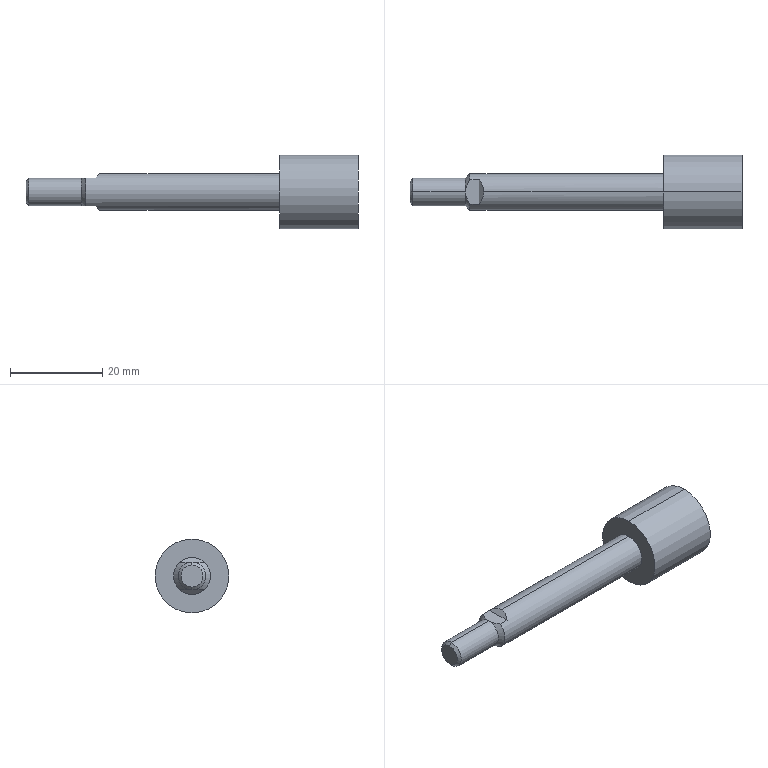Part | STEP file | 001-006-ACQS_16x30_B_30r | 1 solid | 17 faces | box 72 x 16 x 16 mm | volume 5884 mm3 | plane 7 | cylinder 6 | cone 4 | commonest cylinder face diameters 6 x2 8 x2 16 x2
STEP:
#1=CARTESIAN_POINT('',(0.,0.,0.));
#2=DIRECTION('',(0.,0.,1.));
#3=DIRECTION('',(1.,0.,0.));
#4=AXIS2_PLACEMENT_3D('',#1,#2,#3);
#5=CARTESIAN_POINT('',(-3.5,0.,3.));
#6=VERTEX_POINT('',#5);
#7=CARTESIAN_POINT('',(-3.5,0.,-3.));
#8=VERTEX_POINT('',#7);
#9=CARTESIAN_POINT('',(-3.5,0.,0.));
#10=DIRECTION('',(-1.,0.,0.));
#11=DIRECTION('',(0.,0.,1.));
#12=AXIS2_PLACEMENT_3D('',#9,#10,#11);
#13=CIRCLE('',#12,3.);
#14=CARTESIAN_POINT('',(0.,0.,0.));
#15=DIRECTION('',(-1.,0.,0.));
#16=DIRECTION('',(0.,0.,1.));
#17=AXIS2_PLACEMENT_3D('',#14,#15,#16);
#18=CYLINDRICAL_SURFACE('',#17,3.);
#19=CARTESIAN_POINT('',(0.,3.5));
#20=DIRECTION('',(1.,0.));
#21=VECTOR('',#20,1.);
#22=LINE('',#19,#21);
#23=(GEOMETRIC_REPRESENTATION_CONTEXT(2)PARAMETRIC_REPRESENTATION_CONTEXT()REPRESENTATION_CONTEXT('',''));
#24=DEFINITIONAL_REPRESENTATION('',(#22),#23);
#25=PCURVE('',#18,#24);
#26=CARTESIAN_POINT('',(-2.5,0.,0.));
#27=DIRECTION('',(1.,0.,0.));
#28=DIRECTION('',(0.,0.,-1.));
#29=AXIS2_PLACEMENT_3D('',#26,#27,#28);
#30=CONICAL_SURFACE('',#29,4.,0.7854);
#31=CARTESIAN_POINT('',(3.142,-1.));
#32=DIRECTION('',(-1.,0.));
#33=VECTOR('',#32,1.);
#34=LINE('',#31,#33);
#35=(GEOMETRIC_REPRESENTATION_CONTEXT(2)PARAMETRIC_REPRESENTATION_CONTEXT()REPRESENTATION_CONTEXT('',''));
#36=DEFINITIONAL_REPRESENTATION('',(#34),#35);
#37=PCURVE('',#30,#36);
#38=SURFACE_CURVE('',#13,(#25,#37),.PCURVE_S1.);
#39=EDGE_CURVE('',#6,#8,#38,.T.);
#40=ORIENTED_EDGE('',*,*,#39,.T.);
#41=CARTESIAN_POINT('',(-14.886,0.,-3.));
#42=VERTEX_POINT('',#41);
#43=CARTESIAN_POINT('',(0.,0.,-3.));
#44=DIRECTION('',(-1.,0.,0.));
#45=VECTOR('',#44,1.);
#46=LINE('',#43,#45);
#47=CARTESIAN_POINT('',(3.142,0.));
#48=DIRECTION('',(0.,1.));
#49=VECTOR('',#48,1.);
#50=LINE('',#47,#49);
#51=(GEOMETRIC_REPRESENTATION_CONTEXT(2)PARAMETRIC_REPRESENTATION_CONTEXT()REPRESENTATION_CONTEXT('',''));
#52=DEFINITIONAL_REPRESENTATION('',(#50),#51);
#53=PCURVE('',#18,#52);
#54=CARTESIAN_POINT('',(0.,0.,0.));
#55=DIRECTION('',(-1.,0.,0.));
#56=DIRECTION('',(0.,0.,1.));
#57=AXIS2_PLACEMENT_3D('',#54,#55,#56);
#58=CYLINDRICAL_SURFACE('',#57,3.);
#59=CARTESIAN_POINT('',(3.142,0.));
#60=DIRECTION('',(0.,1.));
#61=VECTOR('',#60,1.);
#62=LINE('',#59,#61);
#63=(GEOMETRIC_REPRESENTATION_CONTEXT(2)PARAMETRIC_REPRESENTATION_CONTEXT()REPRESENTATION_CONTEXT('',''));
#64=DEFINITIONAL_REPRESENTATION('',(#62),#63);
#65=PCURVE('',#58,#64);
#66=SURFACE_CURVE('',#46,(#53,#65),.PCURVE_S1.);
#67=EDGE_CURVE('',#8,#42,#66,.T.);
#68=ORIENTED_EDGE('',*,*,#67,.T.);
#69=CARTESIAN_POINT('',(-14.886,0.,3.));
#70=VERTEX_POINT('',#69);
#71=CARTESIAN_POINT('',(-14.886,0.,0.));
#72=DIRECTION('',(-1.,0.,0.));
#73=DIRECTION('',(0.,0.,1.));
#74=AXIS2_PLACEMENT_3D('',#71,#72,#73);
#75=CIRCLE('',#74,3.);
#76=CARTESIAN_POINT('',(0.,14.886));
#77=DIRECTION('',(1.,0.));
#78=VECTOR('',#77,1.);
#79=LINE('',#76,#78);
#80=(GEOMETRIC_REPRESENTATION_CONTEXT(2)PARAMETRIC_REPRESENTATION_CONTEXT()REPRESENTATION_CONTEXT('',''));
#81=DEFINITIONAL_REPRESENTATION('',(#79),#80);
#82=PCURVE('',#18,#81);
#83=CARTESIAN_POINT('',(-14.886,0.,0.));
#84=DIRECTION('',(1.,0.,0.));
#85=DIRECTION('',(0.,0.,-1.));
#86=AXIS2_PLACEMENT_3D('',#83,#84,#85);
#87=CONICAL_SURFACE('',#86,3.,0.7854);
#88=CARTESIAN_POINT('',(3.142,0.));
#89=DIRECTION('',(-1.,0.));
#90=VECTOR('',#89,1.);
#91=LINE('',#88,#90);
#92=(GEOMETRIC_REPRESENTATION_CONTEXT(2)PARAMETRIC_REPRESENTATION_CONTEXT()REPRESENTATION_CONTEXT('',''));
#93=DEFINITIONAL_REPRESENTATION('',(#91),#92);
#94=PCURVE('',#87,#93);
#95=SURFACE_CURVE('',#75,(#82,#94),.PCURVE_S1.);
#96=EDGE_CURVE('',#70,#42,#95,.T.);
#97=ORIENTED_EDGE('',*,*,#96,.F.);
#98=CARTESIAN_POINT('',(0.,0.,3.));
#99=DIRECTION('',(-1.,0.,0.));
#100=VECTOR('',#99,1.);
#101=LINE('',#98,#100);
#102=CARTESIAN_POINT('',(0.,0.));
#103=DIRECTION('',(0.,1.));
#104=VECTOR('',#103,1.);
#105=LINE('',#102,#104);
#106=(GEOMETRIC_REPRESENTATION_CONTEXT(2)PARAMETRIC_REPRESENTATION_CONTEXT()REPRESENTATION_CONTEXT('',''));
#107=DEFINITIONAL_REPRESENTATION('',(#105),#106);
#108=PCURVE('',#18,#107);
#109=CARTESIAN_POINT('',(6.283,0.));
#110=DIRECTION('',(0.,1.));
#111=VECTOR('',#110,1.);
#112=LINE('',#109,#111);
#113=(GEOMETRIC_REPRESENTATION_CONTEXT(2)PARAMETRIC_REPRESENTATION_CONTEXT()REPRESENTATION_CONTEXT('',''));
#114=DEFINITIONAL_REPRESENTATION('',(#112),#113);
#115=PCURVE('',#58,#114);
#116=SURFACE_CURVE('',#101,(#108,#115),.PCURVE_S1.);
#117=EDGE_CURVE('',#6,#70,#116,.T.);
#118=ORIENTED_EDGE('',*,*,#117,.F.);
#119=EDGE_LOOP('',(#40,#68,#97,#118));
#120=FACE_BOUND('',#119,.T.);
#121=ADVANCED_FACE('',(#120),#18,.T.);
#122=CARTESIAN_POINT('',(-15.5,0.,2.386));
#123=VERTEX_POINT('',#122);
#124=CARTESIAN_POINT('',(-15.5,0.,-2.386));
#125=VERTEX_POINT('',#124);
#126=CARTESIAN_POINT('',(-15.5,0.,0.));
#127=DIRECTION('',(-1.,0.,0.));
#128=DIRECTION('',(0.,0.,1.));
#129=AXIS2_PLACEMENT_3D('',#126,#127,#128);
#130=CIRCLE('',#129,2.386);
#131=CARTESIAN_POINT('',(3.142,-0.6135));
#132=DIRECTION('',(-1.,0.));
#133=VECTOR('',#132,1.);
#134=LINE('',#131,#133);
#135=(GEOMETRIC_REPRESENTATION_CONTEXT(2)PARAMETRIC_REPRESENTATION_CONTEXT()REPRESENTATION_CONTEXT('',''));
#136=DEFINITIONAL_REPRESENTATION('',(#134),#135);
#137=PCURVE('',#87,#136);
#138=CARTESIAN_POINT('',(-15.5,0.,0.));
#139=DIRECTION('',(1.,0.,0.));
#140=DIRECTION('',(0.,0.,-1.));
#141=AXIS2_PLACEMENT_3D('',#138,#139,#140);
#142=PLANE('',#141);
#143=CARTESIAN_POINT('',(-2.386,0.));
#144=CARTESIAN_POINT('',(-2.386,4.134));
#145=CARTESIAN_POINT('',(1.193,2.067));
#146=CARTESIAN_POINT('',(4.773,0.));
#147=CARTESIAN_POINT('',(1.193,-2.067));
#148=CARTESIAN_POINT('',(-2.386,-4.134));
#149=CARTESIAN_POINT('',(-2.386,0.));
#150=(BOUNDED_CURVE()B_SPLINE_CURVE(2,(#143,#144,#145,#146,#147,#148,#149),.UNSPECIFIED.,.T.,.F.)B_SPLINE_CURVE_WITH_KNOTS((1,2,2,2,2,1),(-2.094,0.,2.094,4.189,6.283,8.378),.UNSPECIFIED.)CURVE()GEOMETRIC_REPRESENTATION_ITEM()RATIONAL_B_SPLINE_CURVE((1.,0.5,1.,0.5,1.,0.5,1.))REPRESENTATION_ITEM(''));
#151=(GEOMETRIC_REPRESENTATION_CONTEXT(2)PARAMETRIC_REPRESENTATION_CONTEXT()REPRESENTATION_CONTEXT('',''));
#152=DEFINITIONAL_REPRESENTATION('',(#150),#151);
#153=PCURVE('',#142,#152);
#154=SURFACE_CURVE('',#130,(#137,#153),.PCURVE_S1.);
#155=EDGE_CURVE('',#123,#125,#154,.T.);
#156=ORIENTED_EDGE('',*,*,#155,.F.);
#157=CARTESIAN_POINT('',(-14.886,0.,3.));
#158=DIRECTION('',(0.7071,0.,0.7071));
#159=VECTOR('',#158,1.);
#160=LINE('',#157,#159);
#161=CARTESIAN_POINT('',(3.142,0.));
#162=DIRECTION('',(0.,1.));
#163=VECTOR('',#162,1.);
#164=LINE('',#161,#163);
#165=(GEOMETRIC_REPRESENTATION_CONTEXT(2)PARAMETRIC_REPRESENTATION_CONTEXT()REPRESENTATION_CONTEXT('',''));
#166=DEFINITIONAL_REPRESENTATION('',(#164),#165);
#167=PCURVE('',#87,#166);
#168=CARTESIAN_POINT('',(-14.886,0.,0.));
#169=DIRECTION('',(1.,0.,0.));
#170=DIRECTION('',(0.,0.,-1.));
#171=AXIS2_PLACEMENT_3D('',#168,#169,#170);
#172=CONICAL_SURFACE('',#171,3.,0.7854);
#173=CARTESIAN_POINT('',(3.142,0.));
#174=DIRECTION('',(0.,1.));
#175=VECTOR('',#174,1.);
#176=LINE('',#173,#175);
#177=(GEOMETRIC_REPRESENTATION_CONTEXT(2)PARAMETRIC_REPRESENTATION_CONTEXT()REPRESENTATION_CONTEXT('',''));
#178=DEFINITIONAL_REPRESENTATION('',(#176),#177);
#179=PCURVE('',#172,#178);
#180=SURFACE_CURVE('',#160,(#167,#179),.PCURVE_S1.);
#181=EDGE_CURVE('',#123,#70,#180,.T.);
#182=ORIENTED_EDGE('',*,*,#181,.T.);
#183=ORIENTED_EDGE('',*,*,#96,.T.);
#184=CARTESIAN_POINT('',(-14.886,0.,-3.));
#185=DIRECTION('',(0.7071,0.,-0.7071));
#186=VECTOR('',#185,1.);
#187=LINE('',#184,#186);
#188=CARTESIAN_POINT('',(0.,0.));
#189=DIRECTION('',(0.,1.));
#190=VECTOR('',#189,1.);
#191=LINE('',#188,#190);
#192=(GEOMETRIC_REPRESENTATION_CONTEXT(2)PARAMETRIC_REPRESENTATION_CONTEXT()REPRESENTATION_CONTEXT('',''));
#193=DEFINITIONAL_REPRESENTATION('',(#191),#192);
#194=PCURVE('',#87,#193);
#195=CARTESIAN_POINT('',(6.283,0.));
#196=DIRECTION('',(0.,1.));
#197=VECTOR('',#196,1.);
#198=LINE('',#195,#197);
#199=(GEOMETRIC_REPRESENTATION_CONTEXT(2)PARAMETRIC_REPRESENTATION_CONTEXT()REPRESENTATION_CONTEXT('',''));
#200=DEFINITIONAL_REPRESENTATION('',(#198),#199);
#201=PCURVE('',#172,#200);
#202=SURFACE_CURVE('',#187,(#194,#201),.PCURVE_S1.);
#203=EDGE_CURVE('',#125,#42,#202,.T.);
#204=ORIENTED_EDGE('',*,*,#203,.F.);
#205=EDGE_LOOP('',(#156,#182,#183,#204));
#206=FACE_BOUND('',#205,.T.);
#207=ADVANCED_FACE('',(#206),#87,.T.);
#208=CARTESIAN_POINT('',(56.5,0.,8.));
#209=VERTEX_POINT('',#208);
#210=CARTESIAN_POINT('',(56.5,0.,-8.));
#211=VERTEX_POINT('',#210);
#212=CARTESIAN_POINT('',(56.5,0.,0.));
#213=DIRECTION('',(-1.,0.,0.));
#214=DIRECTION('',(0.,0.,1.));
#215=AXIS2_PLACEMENT_3D('',#212,#213,#214);
#216=CIRCLE('',#215,8.);
#217=CARTESIAN_POINT('',(56.5,0.,0.));
#218=DIRECTION('',(-1.,0.,0.));
#219=DIRECTION('',(0.,0.,1.));
#220=AXIS2_PLACEMENT_3D('',#217,#218,#219);
#221=CYLINDRICAL_SURFACE('',#220,8.);
#222=CARTESIAN_POINT('',(0.,0.));
#223=DIRECTION('',(1.,0.));
#224=VECTOR('',#223,1.);
#225=LINE('',#222,#224);
#226=(GEOMETRIC_REPRESENTATION_CONTEXT(2)PARAMETRIC_REPRESENTATION_CONTEXT()REPRESENTATION_CONTEXT('',''));
#227=DEFINITIONAL_REPRESENTATION('',(#225),#226);
#228=PCURVE('',#221,#227);
#229=CARTESIAN_POINT('',(56.5,8.,0.));
#230=DIRECTION('',(-1.,0.,0.));
#231=DIRECTION('',(0.,0.,1.));
#232=AXIS2_PLACEMENT_3D('',#229,#230,#231);
#233=PLANE('',#232);
#234=CARTESIAN_POINT('',(0.,-8.));
#235=DIRECTION('',(1.,0.));
#236=AXIS2_PLACEMENT_2D('',#234,#235);
#237=CIRCLE('',#236,8.);
#238=(GEOMETRIC_REPRESENTATION_CONTEXT(2)PARAMETRIC_REPRESENTATION_CONTEXT()REPRESENTATION_CONTEXT('',''));
#239=DEFINITIONAL_REPRESENTATION('',(#237),#238);
#240=PCURVE('',#233,#239);
#241=SURFACE_CURVE('',#216,(#228,#240),.PCURVE_S1.);
#242=EDGE_CURVE('',#209,#211,#241,.T.);
#243=ORIENTED_EDGE('',*,*,#242,.T.);
#244=CARTESIAN_POINT('',(39.5,0.,-8.));
#245=VERTEX_POINT('',#244);
#246=CARTESIAN_POINT('',(56.5,0.,-8.));
#247=DIRECTION('',(-1.,0.,0.));
#248=VECTOR('',#247,1.);
#249=LINE('',#246,#248);
#250=CARTESIAN_POINT('',(3.142,0.));
#251=DIRECTION('',(0.,1.));
#252=VECTOR('',#251,1.);
#253=LINE('',#250,#252);
#254=(GEOMETRIC_REPRESENTATION_CONTEXT(2)PARAMETRIC_REPRESENTATION_CONTEXT()REPRESENTATION_CONTEXT('',''));
#255=DEFINITIONAL_REPRESENTATION('',(#253),#254);
#256=PCURVE('',#221,#255);
#257=CARTESIAN_POINT('',(56.5,0.,0.));
#258=DIRECTION('',(-1.,0.,0.));
#259=DIRECTION('',(0.,0.,1.));
#260=AXIS2_PLACEMENT_3D('',#257,#258,#259);
#261=CYLINDRICAL_SURFACE('',#260,8.);
#262=CARTESIAN_POINT('',(3.142,0.));
#263=DIRECTION('',(0.,1.));
#264=VECTOR('',#263,1.);
#265=LINE('',#262,#264);
#266=(GEOMETRIC_REPRESENTATION_CONTEXT(2)PARAMETRIC_REPRESENTATION_CONTEXT()REPRESENTATION_CONTEXT('',''));
#267=DEFINITIONAL_REPRESENTATION('',(#265),#266);
#268=PCURVE('',#261,#267);
#269=SURFACE_CURVE('',#249,(#256,#268),.PCURVE_S1.);
#270=EDGE_CURVE('',#211,#245,#269,.T.);
#271=ORIENTED_EDGE('',*,*,#270,.T.);
#272=CARTESIAN_POINT('',(39.5,0.,8.));
#273=VERTEX_POINT('',#272);
#274=CARTESIAN_POINT('',(39.5,0.,0.));
#275=DIRECTION('',(-1.,0.,0.));
#276=DIRECTION('',(0.,0.,1.));
#277=AXIS2_PLACEMENT_3D('',#274,#275,#276);
#278=CIRCLE('',#277,8.);
#279=CARTESIAN_POINT('',(0.,17.));
#280=DIRECTION('',(1.,0.));
#281=VECTOR('',#280,1.);
#282=LINE('',#279,#281);
#283=(GEOMETRIC_REPRESENTATION_CONTEXT(2)PARAMETRIC_REPRESENTATION_CONTEXT()REPRESENTATION_CONTEXT('',''));
#284=DEFINITIONAL_REPRESENTATION('',(#282),#283);
#285=PCURVE('',#221,#284);
#286=CARTESIAN_POINT('',(39.5,4.,0.));
#287=DIRECTION('',(1.,0.,0.));
#288=DIRECTION('',(0.,0.,-1.));
#289=AXIS2_PLACEMENT_3D('',#286,#287,#288);
#290=PLANE('',#289);
#291=CARTESIAN_POINT('',(-8.,-4.));
#292=CARTESIAN_POINT('',(-8.,9.856));
#293=CARTESIAN_POINT('',(4.,2.928));
#294=CARTESIAN_POINT('',(16.,-4.));
#295=CARTESIAN_POINT('',(4.,-10.928));
#296=CARTESIAN_POINT('',(-8.,-17.856));
#297=CARTESIAN_POINT('',(-8.,-4.));
#298=(BOUNDED_CURVE()B_SPLINE_CURVE(2,(#291,#292,#293,#294,#295,#296,#297),.UNSPECIFIED.,.T.,.F.)B_SPLINE_CURVE_WITH_KNOTS((1,2,2,2,2,1),(-2.094,0.,2.094,4.189,6.283,8.378),.UNSPECIFIED.)CURVE()GEOMETRIC_REPRESENTATION_ITEM()RATIONAL_B_SPLINE_CURVE((1.,0.5,1.,0.5,1.,0.5,1.))REPRESENTATION_ITEM(''));
#299=(GEOMETRIC_REPRESENTATION_CONTEXT(2)PARAMETRIC_REPRESENTATION_CONTEXT()REPRESENTATION_CONTEXT('',''));
#300=DEFINITIONAL_REPRESENTATION('',(#298),#299);
#301=PCURVE('',#290,#300);
#302=SURFACE_CURVE('',#278,(#285,#301),.PCURVE_S1.);
#303=EDGE_CURVE('',#273,#245,#302,.T.);
#304=ORIENTED_EDGE('',*,*,#303,.F.);
#305=CARTESIAN_POINT('',(56.5,0.,8.));
#306=DIRECTION('',(-1.,0.,0.));
#307=VECTOR('',#306,1.);
#308=LINE('',#305,#307);
#309=CARTESIAN_POINT('',(0.,0.));
#310=DIRECTION('',(0.,1.));
#311=VECTOR('',#310,1.);
#312=LINE('',#309,#311);
#313=(GEOMETRIC_REPRESENTATION_CONTEXT(2)PARAMETRIC_REPRESENTATION_CONTEXT()REPRESENTATION_CONTEXT('',''));
#314=DEFINITIONAL_REPRESENTATION('',(#312),#313);
#315=PCURVE('',#221,#314);
#316=CARTESIAN_POINT('',(6.283,0.));
#317=DIRECTION('',(0.,1.));
#318=VECTOR('',#317,1.);
#319=LINE('',#316,#318);
#320=(GEOMETRIC_REPRESENTATION_CONTEXT(2)PARAMETRIC_REPRESENTATION_CONTEXT()REPRESENTATION_CONTEXT('',''));
#321=DEFINITIONAL_REPRESENTATION('',(#319),#320);
#322=PCURVE('',#261,#321);
#323=SURFACE_CURVE('',#308,(#315,#322),.PCURVE_S1.);
#324=EDGE_CURVE('',#209,#273,#323,.T.);
#325=ORIENTED_EDGE('',*,*,#324,.F.);
#326=EDGE_LOOP('',(#243,#271,#304,#325));
#327=FACE_BOUND('',#326,.T.);
#328=ADVANCED_FACE('',(#327),#221,.T.);
#329=CARTESIAN_POINT('',(39.5,0.,4.));
#330=VERTEX_POINT('',#329);
#331=CARTESIAN_POINT('',(39.5,0.,-4.));
#332=VERTEX_POINT('',#331);
#333=CARTESIAN_POINT('',(39.5,0.,0.));
#334=DIRECTION('',(-1.,0.,0.));
#335=DIRECTION('',(0.,0.,1.));
#336=AXIS2_PLACEMENT_3D('',#333,#334,#335);
#337=CIRCLE('',#336,4.);
#338=CARTESIAN_POINT('',(56.5,0.,0.));
#339=DIRECTION('',(-1.,0.,0.));
#340=DIRECTION('',(0.,0.,1.));
#341=AXIS2_PLACEMENT_3D('',#338,#339,#340);
#342=CYLINDRICAL_SURFACE('',#341,4.);
#343=CARTESIAN_POINT('',(0.,17.));
#344=DIRECTION('',(1.,0.));
#345=VECTOR('',#344,1.);
#346=LINE('',#343,#345);
#347=(GEOMETRIC_REPRESENTATION_CONTEXT(2)PARAMETRIC_REPRESENTATION_CONTEXT()REPRESENTATION_CONTEXT('',''));
#348=DEFINITIONAL_REPRESENTATION('',(#346),#347);
#349=PCURVE('',#342,#348);
#350=CARTESIAN_POINT('',(-4.,-4.));
#351=CARTESIAN_POINT('',(-4.,2.928));
#352=CARTESIAN_POINT('',(2.,-0.5359));
#353=CARTESIAN_POINT('',(8.,-4.));
#354=CARTESIAN_POINT('',(2.,-7.464));
#355=CARTESIAN_POINT('',(-4.,-10.928));
#356=CARTESIAN_POINT('',(-4.,-4.));
#357=(BOUNDED_CURVE()B_SPLINE_CURVE(2,(#350,#351,#352,#353,#354,#355,#356),.UNSPECIFIED.,.T.,.F.)B_SPLINE_CURVE_WITH_KNOTS((1,2,2,2,2,1),(-2.094,0.,2.094,4.189,6.283,8.378),.UNSPECIFIED.)CURVE()GEOMETRIC_REPRESENTATION_ITEM()RATIONAL_B_SPLINE_CURVE((1.,0.5,1.,0.5,1.,0.5,1.))REPRESENTATION_ITEM(''));
#358=(GEOMETRIC_REPRESENTATION_CONTEXT(2)PARAMETRIC_REPRESENTATION_CONTEXT()REPRESENTATION_CONTEXT('',''));
#359=DEFINITIONAL_REPRESENTATION('',(#357),#358);
#360=PCURVE('',#290,#359);
#361=SURFACE_CURVE('',#337,(#349,#360),.PCURVE_S1.);
#362=EDGE_CURVE('',#330,#332,#361,.T.);
#363=ORIENTED_EDGE('',*,*,#362,.T.);
#364=CARTESIAN_POINT('',(0.5,0.,-4.));
#365=VERTEX_POINT('',#364);
#366=CARTESIAN_POINT('',(56.5,0.,-4.));
#367=DIRECTION('',(-1.,0.,0.));
#368=VECTOR('',#367,1.);
#369=LINE('',#366,#368);
#370=CARTESIAN_POINT('',(3.142,0.));
#371=DIRECTION('',(0.,1.));
#372=VECTOR('',#371,1.);
#373=LINE('',#370,#372);
#374=(GEOMETRIC_REPRESENTATION_CONTEXT(2)PARAMETRIC_REPRESENTATION_CONTEXT()REPRESENTATION_CONTEXT('',''));
#375=DEFINITIONAL_REPRESENTATION('',(#373),#374);
#376=PCURVE('',#342,#375);
#377=CARTESIAN_POINT('',(56.5,0.,0.));
#378=DIRECTION('',(-1.,0.,0.));
#379=DIRECTION('',(0.,0.,1.));
#380=AXIS2_PLACEMENT_3D('',#377,#378,#379);
#381=CYLINDRICAL_SURFACE('',#380,4.);
#382=CARTESIAN_POINT('',(3.142,0.));
#383=DIRECTION('',(0.,1.));
#384=VECTOR('',#383,1.);
#385=LINE('',#382,#384);
#386=(GEOMETRIC_REPRESENTATION_CONTEXT(2)PARAMETRIC_REPRESENTATION_CONTEXT()REPRESENTATION_CONTEXT('',''));
#387=DEFINITIONAL_REPRESENTATION('',(#385),#386);
#388=PCURVE('',#381,#387);
#389=SURFACE_CURVE('',#369,(#376,#388),.PCURVE_S1.);
#390=EDGE_CURVE('',#332,#365,#389,.T.);
#391=ORIENTED_EDGE('',*,*,#390,.T.);
#392=CARTESIAN_POINT('',(-0.5,2.646,-3.));
#393=VERTEX_POINT('',#392);
#394=CARTESIAN_POINT('',(-0.5,2.646,-3.));
#395=CARTESIAN_POINT('',(0.1517,1.907,-3.652));
#396=CARTESIAN_POINT('',(0.5,0.9852,-4.));
#397=CARTESIAN_POINT('',(0.5,0.,-4.));
#398=(BOUNDED_CURVE()B_SPLINE_CURVE(3,(#394,#395,#396,#397),.UNSPECIFIED.,.F.,.F.)B_SPLINE_CURVE_WITH_KNOTS((4,4),(2.419,3.142),.PIECEWISE_BEZIER_KNOTS.)CURVE()GEOMETRIC_REPRESENTATION_ITEM()RATIONAL_B_SPLINE_CURVE((1.,0.9569,0.9569,1.))REPRESENTATION_ITEM(''));
#399=CARTESIAN_POINT('',(2.419,57.));
#400=CARTESIAN_POINT('',(2.43,56.972));
#401=CARTESIAN_POINT('',(2.451,56.916));
#402=CARTESIAN_POINT('',(2.483,56.835));
#403=CARTESIAN_POINT('',(2.516,56.757));
#404=CARTESIAN_POINT('',(2.549,56.682));
#405=CARTESIAN_POINT('',(2.582,56.61));
#406=CARTESIAN_POINT('',(2.615,56.542));
#407=CARTESIAN_POINT('',(2.648,56.478));
#408=CARTESIAN_POINT('',(2.681,56.417));
#409=CARTESIAN_POINT('',(2.714,56.36));
#410=CARTESIAN_POINT('',(2.747,56.307));
#411=CARTESIAN_POINT('',(2.78,56.258));
#412=CARTESIAN_POINT('',(2.813,56.213));
#413=CARTESIAN_POINT('',(2.847,56.172));
#414=CARTESIAN_POINT('',(2.88,56.136));
#415=CARTESIAN_POINT('',(2.913,56.103));
#416=CARTESIAN_POINT('',(2.946,56.076));
#417=CARTESIAN_POINT('',(2.979,56.052));
#418=CARTESIAN_POINT('',(3.012,56.033));
#419=CARTESIAN_POINT('',(3.044,56.018));
#420=CARTESIAN_POINT('',(3.077,56.008));
#421=CARTESIAN_POINT('',(3.109,56.001));
#422=CARTESIAN_POINT('',(3.131,56.));
#423=CARTESIAN_POINT('',(3.142,56.));
#424=B_SPLINE_CURVE_WITH_KNOTS('',3,(#399,#400,#401,#402,#403,#404,#405,#406,#407,#408,#409,#410,#411,#412,#413,#414,#415,#416,#417,#418,#419,#420,#421,#422,#423),.UNSPECIFIED.,.F.,.F.,(4,1,1,1,1,1,1,1,1,1,1,1,1,1,1,1,1,1,1,1,1,1,4),(2.419,2.452,2.485,2.517,2.55,2.583,2.616,2.649,2.682,2.715,2.747,2.78,2.813,2.846,2.879,2.912,2.944,2.977,3.01,3.043,3.076,3.109,3.142),.QUASI_UNIFORM_KNOTS.);
#425=(GEOMETRIC_REPRESENTATION_CONTEXT(2)PARAMETRIC_REPRESENTATION_CONTEXT()REPRESENTATION_CONTEXT('',''));
#426=DEFINITIONAL_REPRESENTATION('',(#424),#425);
#427=PCURVE('',#342,#426);
#428=CARTESIAN_POINT('',(-0.5,6.,-3.));
#429=DIRECTION('',(-0.7071,0.,-0.7071));
#430=DIRECTION('',(-0.7071,0.,0.7071));
#431=AXIS2_PLACEMENT_3D('',#428,#429,#430);
#432=PLANE('',#431);
#433=CARTESIAN_POINT('',(0.,-3.354));
#434=CARTESIAN_POINT('',(-0.9216,-4.093));
#435=CARTESIAN_POINT('',(-1.414,-5.015));
#436=CARTESIAN_POINT('',(-1.414,-6.));
#437=(BOUNDED_CURVE()B_SPLINE_CURVE(3,(#433,#434,#435,#436),.UNSPECIFIED.,.F.,.F.)B_SPLINE_CURVE_WITH_KNOTS((4,4),(2.419,3.142),.PIECEWISE_BEZIER_KNOTS.)CURVE()GEOMETRIC_REPRESENTATION_ITEM()RATIONAL_B_SPLINE_CURVE((1.,0.9569,0.9569,1.))REPRESENTATION_ITEM(''));
#438=(GEOMETRIC_REPRESENTATION_CONTEXT(2)PARAMETRIC_REPRESENTATION_CONTEXT()REPRESENTATION_CONTEXT('',''));
#439=DEFINITIONAL_REPRESENTATION('',(#437),#438);
#440=PCURVE('',#432,#439);
#441=SURFACE_CURVE('',#398,(#427,#440),.PCURVE_S1.);
#442=EDGE_CURVE('',#393,#365,#441,.T.);
#443=ORIENTED_EDGE('',*,*,#442,.F.);
#444=CARTESIAN_POINT('',(-2.5,2.646,-3.));
#445=VERTEX_POINT('',#444);
#446=CARTESIAN_POINT('',(56.5,2.646,-3.));
#447=DIRECTION('',(1.,0.,0.));
#448=VECTOR('',#447,1.);
#449=LINE('',#446,#448);
#450=CARTESIAN_POINT('',(2.419,0.));
#451=DIRECTION('',(0.,-1.));
#452=VECTOR('',#451,1.);
#453=LINE('',#450,#452);
#454=(GEOMETRIC_REPRESENTATION_CONTEXT(2)PARAMETRIC_REPRESENTATION_CONTEXT()REPRESENTATION_CONTEXT('',''));
#455=DEFINITIONAL_REPRESENTATION('',(#453),#454);
#456=PCURVE('',#342,#455);
#457=CARTESIAN_POINT('',(-3.5,6.,-3.));
#458=DIRECTION('',(0.,0.,-1.));
#459=DIRECTION('',(-1.,0.,0.));
#460=AXIS2_PLACEMENT_3D('',#457,#458,#459);
#461=PLANE('',#460);
#462=CARTESIAN_POINT('',(-60.,-3.354));
#463=DIRECTION('',(-1.,0.));
#464=VECTOR('',#463,1.);
#465=LINE('',#462,#464);
#466=(GEOMETRIC_REPRESENTATION_CONTEXT(2)PARAMETRIC_REPRESENTATION_CONTEXT()REPRESENTATION_CONTEXT('',''));
#467=DEFINITIONAL_REPRESENTATION('',(#465),#466);
#468=PCURVE('',#461,#467);
#469=SURFACE_CURVE('',#449,(#456,#468),.PCURVE_S1.);
#470=EDGE_CURVE('',#445,#393,#469,.T.);
#471=ORIENTED_EDGE('',*,*,#470,.F.);
#472=CARTESIAN_POINT('',(-2.5,2.646,3.));
#473=VERTEX_POINT('',#472);
#474=CARTESIAN_POINT('',(-2.5,0.,0.));
#475=DIRECTION('',(-1.,0.,0.));
#476=DIRECTION('',(0.,0.,1.));
#477=AXIS2_PLACEMENT_3D('',#474,#475,#476);
#478=CIRCLE('',#477,4.);
#479=CARTESIAN_POINT('',(0.,59.));
#480=DIRECTION('',(1.,0.));
#481=VECTOR('',#480,1.);
#482=LINE('',#479,#481);
#483=(GEOMETRIC_REPRESENTATION_CONTEXT(2)PARAMETRIC_REPRESENTATION_CONTEXT()REPRESENTATION_CONTEXT('',''));
#484=DEFINITIONAL_REPRESENTATION('',(#482),#483);
#485=PCURVE('',#342,#484);
#486=CARTESIAN_POINT('',(3.142,0.));
#487=DIRECTION('',(-1.,0.));
#488=VECTOR('',#487,1.);
#489=LINE('',#486,#488);
#490=(GEOMETRIC_REPRESENTATION_CONTEXT(2)PARAMETRIC_REPRESENTATION_CONTEXT()REPRESENTATION_CONTEXT('',''));
#491=DEFINITIONAL_REPRESENTATION('',(#489),#490);
#492=PCURVE('',#30,#491);
#493=SURFACE_CURVE('',#478,(#485,#492),.PCURVE_S1.);
#494=EDGE_CURVE('',#473,#445,#493,.T.);
#495=ORIENTED_EDGE('',*,*,#494,.F.);
#496=CARTESIAN_POINT('',(-0.5,2.646,3.));
#497=VERTEX_POINT('',#496);
#498=CARTESIAN_POINT('',(56.5,2.646,3.));
#499=DIRECTION('',(-1.,0.,0.));
#500=VECTOR('',#499,1.);
#501=LINE('',#498,#500);
#502=CARTESIAN_POINT('',(0.7227,0.));
#503=DIRECTION('',(0.,1.));
#504=VECTOR('',#503,1.);
#505=LINE('',#502,#504);
#506=(GEOMETRIC_REPRESENTATION_CONTEXT(2)PARAMETRIC_REPRESENTATION_CONTEXT()REPRESENTATION_CONTEXT('',''));
#507=DEFINITIONAL_REPRESENTATION('',(#505),#506);
#508=PCURVE('',#342,#507);
#509=CARTESIAN_POINT('',(-0.5,6.,3.));
#510=DIRECTION('',(0.,0.,1.));
#511=DIRECTION('',(1.,0.,0.));
#512=AXIS2_PLACEMENT_3D('',#509,#510,#511);
#513=PLANE('',#512);
#514=CARTESIAN_POINT('',(57.,-3.354));
#515=DIRECTION('',(-1.,0.));
#516=VECTOR('',#515,1.);
#517=LINE('',#514,#516);
#518=(GEOMETRIC_REPRESENTATION_CONTEXT(2)PARAMETRIC_REPRESENTATION_CONTEXT()REPRESENTATION_CONTEXT('',''));
#519=DEFINITIONAL_REPRESENTATION('',(#517),#518);
#520=PCURVE('',#513,#519);
#521=SURFACE_CURVE('',#501,(#508,#520),.PCURVE_S1.);
#522=EDGE_CURVE('',#497,#473,#521,.T.);
#523=ORIENTED_EDGE('',*,*,#522,.F.);
#524=CARTESIAN_POINT('',(0.5,0.,4.));
#525=VERTEX_POINT('',#524);
#526=CARTESIAN_POINT('',(0.5,0.,4.));
#527=CARTESIAN_POINT('',(0.5,0.9852,4.));
#528=CARTESIAN_POINT('',(0.1517,1.907,3.652));
#529=CARTESIAN_POINT('',(-0.5,2.646,3.));
#530=(BOUNDED_CURVE()B_SPLINE_CURVE(3,(#526,#527,#528,#529),.UNSPECIFIED.,.F.,.F.)B_SPLINE_CURVE_WITH_KNOTS((4,4),(3.142,3.864),.PIECEWISE_BEZIER_KNOTS.)CURVE()GEOMETRIC_REPRESENTATION_ITEM()RATIONAL_B_SPLINE_CURVE((1.,0.9569,0.9569,1.))REPRESENTATION_ITEM(''));
#531=CARTESIAN_POINT('',(0.,56.));
#532=CARTESIAN_POINT('',(0.01071,56.));
#533=CARTESIAN_POINT('',(0.0322,56.001));
#534=CARTESIAN_POINT('',(0.06461,56.008));
#535=CARTESIAN_POINT('',(0.09718,56.018));
#536=CARTESIAN_POINT('',(0.1299,56.033));
#537=CARTESIAN_POINT('',(0.1627,56.052));
#538=CARTESIAN_POINT('',(0.1957,56.076));
#539=CARTESIAN_POINT('',(0.2287,56.103));
#540=CARTESIAN_POINT('',(0.2618,56.136));
#541=CARTESIAN_POINT('',(0.295,56.172));
#542=CARTESIAN_POINT('',(0.3282,56.213));
#543=CARTESIAN_POINT('',(0.3614,56.258));
#544=CARTESIAN_POINT('',(0.3946,56.307));
#545=CARTESIAN_POINT('',(0.4278,56.36));
#546=CARTESIAN_POINT('',(0.4609,56.417));
#547=CARTESIAN_POINT('',(0.494,56.478));
#548=CARTESIAN_POINT('',(0.5271,56.542));
#549=CARTESIAN_POINT('',(0.56,56.61));
#550=CARTESIAN_POINT('',(0.5928,56.682));
#551=CARTESIAN_POINT('',(0.6256,56.757));
#552=CARTESIAN_POINT('',(0.6581,56.835));
#553=CARTESIAN_POINT('',(0.6905,56.916));
#554=CARTESIAN_POINT('',(0.712,56.972));
#555=CARTESIAN_POINT('',(0.7227,57.));
#556=B_SPLINE_CURVE_WITH_KNOTS('',3,(#531,#532,#533,#534,#535,#536,#537,#538,#539,#540,#541,#542,#543,#544,#545,#546,#547,#548,#549,#550,#551,#552,#553,#554,#555),.UNSPECIFIED.,.F.,.F.,(4,1,1,1,1,1,1,1,1,1,1,1,1,1,1,1,1,1,1,1,1,1,4),(3.142,3.174,3.207,3.24,3.273,3.306,3.339,3.372,3.404,3.437,3.47,3.503,3.536,3.569,3.602,3.634,3.667,3.7,3.733,3.766,3.799,3.831,3.864),.QUASI_UNIFORM_KNOTS.);
#557=(GEOMETRIC_REPRESENTATION_CONTEXT(2)PARAMETRIC_REPRESENTATION_CONTEXT()REPRESENTATION_CONTEXT('',''));
#558=DEFINITIONAL_REPRESENTATION('',(#556),#557);
#559=PCURVE('',#342,#558);
#560=CARTESIAN_POINT('',(19.5,6.,23.));
#561=DIRECTION('',(-0.7071,0.,0.7071));
#562=DIRECTION('',(0.7071,0.,0.7071));
#563=AXIS2_PLACEMENT_3D('',#560,#561,#562);
#564=PLANE('',#563);
#565=CARTESIAN_POINT('',(-26.87,-6.));
#566=CARTESIAN_POINT('',(-26.87,-5.015));
#567=CARTESIAN_POINT('',(-27.363,-4.093));
#568=CARTESIAN_POINT('',(-28.284,-3.354));
#569=(BOUNDED_CURVE()B_SPLINE_CURVE(3,(#565,#566,#567,#568),.UNSPECIFIED.,.F.,.F.)B_SPLINE_CURVE_WITH_KNOTS((4,4),(3.142,3.864),.PIECEWISE_BEZIER_KNOTS.)CURVE()GEOMETRIC_REPRESENTATION_ITEM()RATIONAL_B_SPLINE_CURVE((1.,0.9569,0.9569,1.))REPRESENTATION_ITEM(''));
#570=(GEOMETRIC_REPRESENTATION_CONTEXT(2)PARAMETRIC_REPRESENTATION_CONTEXT()REPRESENTATION_CONTEXT('',''));
#571=DEFINITIONAL_REPRESENTATION('',(#569),#570);
#572=PCURVE('',#564,#571);
#573=SURFACE_CURVE('',#530,(#559,#572),.PCURVE_S1.);
#574=EDGE_CURVE('',#525,#497,#573,.T.);
#575=ORIENTED_EDGE('',*,*,#574,.F.);
#576=CARTESIAN_POINT('',(56.5,0.,4.));
#577=DIRECTION('',(-1.,0.,0.));
#578=VECTOR('',#577,1.);
#579=LINE('',#576,#578);
#580=CARTESIAN_POINT('',(0.,0.));
#581=DIRECTION('',(0.,1.));
#582=VECTOR('',#581,1.);
#583=LINE('',#580,#582);
#584=(GEOMETRIC_REPRESENTATION_CONTEXT(2)PARAMETRIC_REPRESENTATION_CONTEXT()REPRESENTATION_CONTEXT('',''));
#585=DEFINITIONAL_REPRESENTATION('',(#583),#584);
#586=PCURVE('',#342,#585);
#587=CARTESIAN_POINT('',(6.283,0.));
#588=DIRECTION('',(0.,1.));
#589=VECTOR('',#588,1.);
#590=LINE('',#587,#589);
#591=(GEOMETRIC_REPRESENTATION_CONTEXT(2)PARAMETRIC_REPRESENTATION_CONTEXT()REPRESENTATION_CONTEXT('',''));
#592=DEFINITIONAL_REPRESENTATION('',(#590),#591);
#593=PCURVE('',#381,#592);
#594=SURFACE_CURVE('',#579,(#586,#593),.PCURVE_S1.);
#595=EDGE_CURVE('',#330,#525,#594,.T.);
#596=ORIENTED_EDGE('',*,*,#595,.F.);
#597=EDGE_LOOP('',(#363,#391,#443,#471,#495,#523,#575,#596));
#598=FACE_BOUND('',#597,.T.);
#599=ADVANCED_FACE('',(#598),#342,.T.);
#600=ORIENTED_EDGE('',*,*,#390,.F.);
#601=CARTESIAN_POINT('',(39.5,0.,0.));
#602=DIRECTION('',(-1.,0.,0.));
#603=DIRECTION('',(0.,0.,1.));
#604=AXIS2_PLACEMENT_3D('',#601,#602,#603);
#605=CIRCLE('',#604,4.);
#606=CARTESIAN_POINT('',(0.,17.));
#607=DIRECTION('',(1.,0.));
#608=VECTOR('',#607,1.);
#609=LINE('',#606,#608);
#610=(GEOMETRIC_REPRESENTATION_CONTEXT(2)PARAMETRIC_REPRESENTATION_CONTEXT()REPRESENTATION_CONTEXT('',''));
#611=DEFINITIONAL_REPRESENTATION('',(#609),#610);
#612=PCURVE('',#381,#611);
#613=CARTESIAN_POINT('',(-4.,-4.));
#614=CARTESIAN_POINT('',(-4.,2.928));
#615=CARTESIAN_POINT('',(2.,-0.5359));
#616=CARTESIAN_POINT('',(8.,-4.));
#617=CARTESIAN_POINT('',(2.,-7.464));
#618=CARTESIAN_POINT('',(-4.,-10.928));
#619=CARTESIAN_POINT('',(-4.,-4.));
#620=(BOUNDED_CURVE()B_SPLINE_CURVE(2,(#613,#614,#615,#616,#617,#618,#619),.UNSPECIFIED.,.T.,.F.)B_SPLINE_CURVE_WITH_KNOTS((1,2,2,2,2,1),(-2.094,0.,2.094,4.189,6.283,8.378),.UNSPECIFIED.)CURVE()GEOMETRIC_REPRESENTATION_ITEM()RATIONAL_B_SPLINE_CURVE((1.,0.5,1.,0.5,1.,0.5,1.))REPRESENTATION_ITEM(''));
#621=(GEOMETRIC_REPRESENTATION_CONTEXT(2)PARAMETRIC_REPRESENTATION_CONTEXT()REPRESENTATION_CONTEXT('',''));
#622=DEFINITIONAL_REPRESENTATION('',(#620),#621);
#623=PCURVE('',#290,#622);
#624=SURFACE_CURVE('',#605,(#612,#623),.PCURVE_S1.);
#625=EDGE_CURVE('',#332,#330,#624,.T.);
#626=ORIENTED_EDGE('',*,*,#625,.T.);
#627=ORIENTED_EDGE('',*,*,#595,.T.);
#628=CARTESIAN_POINT('',(-0.5,-2.646,3.));
#629=VERTEX_POINT('',#628);
#630=CARTESIAN_POINT('',(-0.5,-2.646,3.));
#631=CARTESIAN_POINT('',(0.1517,-1.907,3.652));
#632=CARTESIAN_POINT('',(0.5,-0.9852,4.));
#633=CARTESIAN_POINT('',(0.5,0.,4.));
#634=(BOUNDED_CURVE()B_SPLINE_CURVE(3,(#630,#631,#632,#633),.UNSPECIFIED.,.F.,.F.)B_SPLINE_CURVE_WITH_KNOTS((4,4),(2.419,3.142),.PIECEWISE_BEZIER_KNOTS.)CURVE()GEOMETRIC_REPRESENTATION_ITEM()RATIONAL_B_SPLINE_CURVE((1.,0.9569,0.9569,1.))REPRESENTATION_ITEM(''));
#635=CARTESIAN_POINT('',(5.56,57.));
#636=CARTESIAN_POINT('',(5.571,56.972));
#637=CARTESIAN_POINT('',(5.593,56.916));
#638=CARTESIAN_POINT('',(5.625,56.835));
#639=CARTESIAN_POINT('',(5.658,56.757));
#640=CARTESIAN_POINT('',(5.69,56.682));
#641=CARTESIAN_POINT('',(5.723,56.61));
#642=CARTESIAN_POINT('',(5.756,56.542));
#643=CARTESIAN_POINT('',(5.789,56.478));
#644=CARTESIAN_POINT('',(5.822,56.417));
#645=CARTESIAN_POINT('',(5.855,56.36));
#646=CARTESIAN_POINT('',(5.889,56.307));
#647=CARTESIAN_POINT('',(5.922,56.258));
#648=CARTESIAN_POINT('',(5.955,56.213));
#649=CARTESIAN_POINT('',(5.988,56.172));
#650=CARTESIAN_POINT('',(6.021,56.136));
#651=CARTESIAN_POINT('',(6.054,56.103));
#652=CARTESIAN_POINT('',(6.088,56.076));
#653=CARTESIAN_POINT('',(6.12,56.052));
#654=CARTESIAN_POINT('',(6.153,56.033));
#655=CARTESIAN_POINT('',(6.186,56.018));
#656=CARTESIAN_POINT('',(6.219,56.008));
#657=CARTESIAN_POINT('',(6.251,56.001));
#658=CARTESIAN_POINT('',(6.272,56.));
#659=CARTESIAN_POINT('',(6.283,56.));
#660=B_SPLINE_CURVE_WITH_KNOTS('',3,(#635,#636,#637,#638,#639,#640,#641,#642,#643,#644,#645,#646,#647,#648,#649,#650,#651,#652,#653,#654,#655,#656,#657,#658,#659),.UNSPECIFIED.,.F.,.F.,(4,1,1,1,1,1,1,1,1,1,1,1,1,1,1,1,1,1,1,1,1,1,4),(2.419,2.452,2.485,2.517,2.55,2.583,2.616,2.649,2.682,2.715,2.747,2.78,2.813,2.846,2.879,2.912,2.944,2.977,3.01,3.043,3.076,3.109,3.142),.QUASI_UNIFORM_KNOTS.);
#661=(GEOMETRIC_REPRESENTATION_CONTEXT(2)PARAMETRIC_REPRESENTATION_CONTEXT()REPRESENTATION_CONTEXT('',''));
#662=DEFINITIONAL_REPRESENTATION('',(#660),#661);
#663=PCURVE('',#381,#662);
#664=CARTESIAN_POINT('',(-28.284,-8.646));
#665=CARTESIAN_POINT('',(-27.363,-7.907));
#666=CARTESIAN_POINT('',(-26.87,-6.985));
#667=CARTESIAN_POINT('',(-26.87,-6.));
#668=(BOUNDED_CURVE()B_SPLINE_CURVE(3,(#664,#665,#666,#667),.UNSPECIFIED.,.F.,.F.)B_SPLINE_CURVE_WITH_KNOTS((4,4),(2.419,3.142),.PIECEWISE_BEZIER_KNOTS.)CURVE()GEOMETRIC_REPRESENTATION_ITEM()RATIONAL_B_SPLINE_CURVE((1.,0.9569,0.9569,1.))REPRESENTATION_ITEM(''));
#669=(GEOMETRIC_REPRESENTATION_CONTEXT(2)PARAMETRIC_REPRESENTATION_CONTEXT()REPRESENTATION_CONTEXT('',''));
#670=DEFINITIONAL_REPRESENTATION('',(#668),#669);
#671=PCURVE('',#564,#670);
#672=SURFACE_CURVE('',#634,(#663,#671),.PCURVE_S1.);
#673=EDGE_CURVE('',#629,#525,#672,.T.);
#674=ORIENTED_EDGE('',*,*,#673,.F.);
#675=CARTESIAN_POINT('',(-2.5,-2.646,3.));
#676=VERTEX_POINT('',#675);
#677=CARTESIAN_POINT('',(56.5,-2.646,3.));
#678=DIRECTION('',(1.,0.,0.));
#679=VECTOR('',#678,1.);
#680=LINE('',#677,#679);
#681=CARTESIAN_POINT('',(5.56,0.));
#682=DIRECTION('',(0.,-1.));
#683=VECTOR('',#682,1.);
#684=LINE('',#681,#683);
#685=(GEOMETRIC_REPRESENTATION_CONTEXT(2)PARAMETRIC_REPRESENTATION_CONTEXT()REPRESENTATION_CONTEXT('',''));
#686=DEFINITIONAL_REPRESENTATION('',(#684),#685);
#687=PCURVE('',#381,#686);
#688=CARTESIAN_POINT('',(57.,-8.646));
#689=DIRECTION('',(1.,0.));
#690=VECTOR('',#689,1.);
#691=LINE('',#688,#690);
#692=(GEOMETRIC_REPRESENTATION_CONTEXT(2)PARAMETRIC_REPRESENTATION_CONTEXT()REPRESENTATION_CONTEXT('',''));
#693=DEFINITIONAL_REPRESENTATION('',(#691),#692);
#694=PCURVE('',#513,#693);
#695=SURFACE_CURVE('',#680,(#687,#694),.PCURVE_S1.);
#696=EDGE_CURVE('',#676,#629,#695,.T.);
#697=ORIENTED_EDGE('',*,*,#696,.F.);
#698=CARTESIAN_POINT('',(-2.5,-2.646,-3.));
#699=VERTEX_POINT('',#698);
#700=CARTESIAN_POINT('',(-2.5,0.,0.));
#701=DIRECTION('',(-1.,0.,0.));
#702=DIRECTION('',(0.,0.,1.));
#703=AXIS2_PLACEMENT_3D('',#700,#701,#702);
#704=CIRCLE('',#703,4.);
#705=CARTESIAN_POINT('',(0.,59.));
#706=DIRECTION('',(1.,0.));
#707=VECTOR('',#706,1.);
#708=LINE('',#705,#707);
#709=(GEOMETRIC_REPRESENTATION_CONTEXT(2)PARAMETRIC_REPRESENTATION_CONTEXT()REPRESENTATION_CONTEXT('',''));
#710=DEFINITIONAL_REPRESENTATION('',(#708),#709);
#711=PCURVE('',#381,#710);
#712=CARTESIAN_POINT('',(-2.5,0.,0.));
#713=DIRECTION('',(1.,0.,0.));
#714=DIRECTION('',(0.,0.,-1.));
#715=AXIS2_PLACEMENT_3D('',#712,#713,#714);
#716=CONICAL_SURFACE('',#715,4.,0.7854);
#717=CARTESIAN_POINT('',(9.425,0.));
#718=DIRECTION('',(-1.,0.));
#719=VECTOR('',#718,1.);
#720=LINE('',#717,#719);
#721=(GEOMETRIC_REPRESENTATION_CONTEXT(2)PARAMETRIC_REPRESENTATION_CONTEXT()REPRESENTATION_CONTEXT('',''));
#722=DEFINITIONAL_REPRESENTATION('',(#720),#721);
#723=PCURVE('',#716,#722);
#724=SURFACE_CURVE('',#704,(#711,#723),.PCURVE_S1.);
#725=EDGE_CURVE('',#699,#676,#724,.T.);
#726=ORIENTED_EDGE('',*,*,#725,.F.);
#727=CARTESIAN_POINT('',(-0.5,-2.646,-3.));
#728=VERTEX_POINT('',#727);
#729=CARTESIAN_POINT('',(56.5,-2.646,-3.));
#730=DIRECTION('',(-1.,0.,0.));
#731=VECTOR('',#730,1.);
#732=LINE('',#729,#731);
#733=CARTESIAN_POINT('',(3.864,0.));
#734=DIRECTION('',(0.,1.));
#735=VECTOR('',#734,1.);
#736=LINE('',#733,#735);
#737=(GEOMETRIC_REPRESENTATION_CONTEXT(2)PARAMETRIC_REPRESENTATION_CONTEXT()REPRESENTATION_CONTEXT('',''));
#738=DEFINITIONAL_REPRESENTATION('',(#736),#737);
#739=PCURVE('',#381,#738);
#740=CARTESIAN_POINT('',(-60.,-8.646));
#741=DIRECTION('',(1.,0.));
#742=VECTOR('',#741,1.);
#743=LINE('',#740,#742);
#744=(GEOMETRIC_REPRESENTATION_CONTEXT(2)PARAMETRIC_REPRESENTATION_CONTEXT()REPRESENTATION_CONTEXT('',''));
#745=DEFINITIONAL_REPRESENTATION('',(#743),#744);
#746=PCURVE('',#461,#745);
#747=SURFACE_CURVE('',#732,(#739,#746),.PCURVE_S1.);
#748=EDGE_CURVE('',#728,#699,#747,.T.);
#749=ORIENTED_EDGE('',*,*,#748,.F.);
#750=CARTESIAN_POINT('',(0.5,0.,-4.));
#751=CARTESIAN_POINT('',(0.5,-0.9852,-4.));
#752=CARTESIAN_POINT('',(0.1517,-1.907,-3.652));
#753=CARTESIAN_POINT('',(-0.5,-2.646,-3.));
#754=(BOUNDED_CURVE()B_SPLINE_CURVE(3,(#750,#751,#752,#753),.UNSPECIFIED.,.F.,.F.)B_SPLINE_CURVE_WITH_KNOTS((4,4),(3.142,3.864),.PIECEWISE_BEZIER_KNOTS.)CURVE()GEOMETRIC_REPRESENTATION_ITEM()RATIONAL_B_SPLINE_CURVE((1.,0.9569,0.9569,1.))REPRESENTATION_ITEM(''));
#755=CARTESIAN_POINT('',(3.142,56.));
#756=CARTESIAN_POINT('',(3.152,56.));
#757=CARTESIAN_POINT('',(3.174,56.001));
#758=CARTESIAN_POINT('',(3.206,56.008));
#759=CARTESIAN_POINT('',(3.239,56.018));
#760=CARTESIAN_POINT('',(3.271,56.033));
#761=CARTESIAN_POINT('',(3.304,56.052));
#762=CARTESIAN_POINT('',(3.337,56.076));
#763=CARTESIAN_POINT('',(3.37,56.103));
#764=CARTESIAN_POINT('',(3.403,56.136));
#765=CARTESIAN_POINT('',(3.437,56.172));
#766=CARTESIAN_POINT('',(3.47,56.213));
#767=CARTESIAN_POINT('',(3.503,56.258));
#768=CARTESIAN_POINT('',(3.536,56.307));
#769=CARTESIAN_POINT('',(3.569,56.36));
#770=CARTESIAN_POINT('',(3.603,56.417));
#771=CARTESIAN_POINT('',(3.636,56.478));
#772=CARTESIAN_POINT('',(3.669,56.542));
#773=CARTESIAN_POINT('',(3.702,56.61));
#774=CARTESIAN_POINT('',(3.734,56.682));
#775=CARTESIAN_POINT('',(3.767,56.757));
#776=CARTESIAN_POINT('',(3.8,56.835));
#777=CARTESIAN_POINT('',(3.832,56.916));
#778=CARTESIAN_POINT('',(3.854,56.972));
#779=CARTESIAN_POINT('',(3.864,57.));
#780=B_SPLINE_CURVE_WITH_KNOTS('',3,(#755,#756,#757,#758,#759,#760,#761,#762,#763,#764,#765,#766,#767,#768,#769,#770,#771,#772,#773,#774,#775,#776,#777,#778,#779),.UNSPECIFIED.,.F.,.F.,(4,1,1,1,1,1,1,1,1,1,1,1,1,1,1,1,1,1,1,1,1,1,4),(3.142,3.174,3.207,3.24,3.273,3.306,3.339,3.372,3.404,3.437,3.47,3.503,3.536,3.569,3.602,3.634,3.667,3.7,3.733,3.766,3.799,3.831,3.864),.QUASI_UNIFORM_KNOTS.);
#781=(GEOMETRIC_REPRESENTATION_CONTEXT(2)PARAMETRIC_REPRESENTATION_CONTEXT()REPRESENTATION_CONTEXT('',''));
#782=DEFINITIONAL_REPRESENTATION('',(#780),#781);
#783=PCURVE('',#381,#782);
#784=CARTESIAN_POINT('',(-1.414,-6.));
#785=CARTESIAN_POINT('',(-1.414,-6.985));
#786=CARTESIAN_POINT('',(-0.9216,-7.907));
#787=CARTESIAN_POINT('',(0.,-8.646));
#788=(BOUNDED_CURVE()B_SPLINE_CURVE(3,(#784,#785,#786,#787),.UNSPECIFIED.,.F.,.F.)B_SPLINE_CURVE_WITH_KNOTS((4,4),(3.142,3.864),.PIECEWISE_BEZIER_KNOTS.)CURVE()GEOMETRIC_REPRESENTATION_ITEM()RATIONAL_B_SPLINE_CURVE((1.,0.9569,0.9569,1.))REPRESENTATION_ITEM(''));
#789=(GEOMETRIC_REPRESENTATION_CONTEXT(2)PARAMETRIC_REPRESENTATION_CONTEXT()REPRESENTATION_CONTEXT('',''));
#790=DEFINITIONAL_REPRESENTATION('',(#788),#789);
#791=PCURVE('',#432,#790);
#792=SURFACE_CURVE('',#754,(#783,#791),.PCURVE_S1.);
#793=EDGE_CURVE('',#365,#728,#792,.T.);
#794=ORIENTED_EDGE('',*,*,#793,.F.);
#795=EDGE_LOOP('',(#600,#626,#627,#674,#697,#726,#749,#794));
#796=FACE_BOUND('',#795,.T.);
#797=ADVANCED_FACE('',(#796),#381,.T.);
#798=CARTESIAN_POINT('',(-2.5,2.646,3.));
#799=CARTESIAN_POINT('',(-2.763,2.248,3.));
#800=CARTESIAN_POINT('',(-3.004,1.838,3.));
#801=CARTESIAN_POINT('',(-3.282,1.181,3.));
#802=CARTESIAN_POINT('',(-3.361,0.9534,3.));
#803=CARTESIAN_POINT('',(-3.471,0.4787,3.));
#804=CARTESIAN_POINT('',(-3.5,0.24,3.));
#805=CARTESIAN_POINT('',(-3.5,0.,3.));
#806=B_SPLINE_CURVE_WITH_KNOTS('',3,(#798,#799,#800,#801,#802,#803,#804,#805),.UNSPECIFIED.,.F.,.F.,(4,2,2,4),(0.01212,0.01356,0.01427,0.01499),.UNSPECIFIED.);
#807=CARTESIAN_POINT('',(2.419,0.));
#808=CARTESIAN_POINT('',(2.426,-0.02393));
#809=CARTESIAN_POINT('',(2.439,-0.0714));
#810=CARTESIAN_POINT('',(2.461,-0.1413));
#811=CARTESIAN_POINT('',(2.484,-0.2098));
#812=CARTESIAN_POINT('',(2.507,-0.2767));
#813=CARTESIAN_POINT('',(2.532,-0.3419));
#814=CARTESIAN_POINT('',(2.558,-0.4054));
#815=CARTESIAN_POINT('',(2.585,-0.4669));
#816=CARTESIAN_POINT('',(2.613,-0.5262));
#817=CARTESIAN_POINT('',(2.642,-0.5833));
#818=CARTESIAN_POINT('',(2.673,-0.6379));
#819=CARTESIAN_POINT('',(2.705,-0.6899));
#820=CARTESIAN_POINT('',(2.738,-0.739));
#821=CARTESIAN_POINT('',(2.773,-0.785));
#822=CARTESIAN_POINT('',(2.81,-0.8275));
#823=CARTESIAN_POINT('',(2.847,-0.8663));
#824=CARTESIAN_POINT('',(2.887,-0.9009));
#825=CARTESIAN_POINT('',(2.928,-0.931));
#826=CARTESIAN_POINT('',(2.969,-0.9559));
#827=CARTESIAN_POINT('',(3.012,-0.9754));
#828=CARTESIAN_POINT('',(3.055,-0.9895));
#829=CARTESIAN_POINT('',(3.098,-0.9981));
#830=CARTESIAN_POINT('',(3.127,-1.));
#831=CARTESIAN_POINT('',(3.142,-1.));
#832=B_SPLINE_CURVE_WITH_KNOTS('',3,(#807,#808,#809,#810,#811,#812,#813,#814,#815,#816,#817,#818,#819,#820,#821,#822,#823,#824,#825,#826,#827,#828,#829,#830,#831),.UNSPECIFIED.,.F.,.F.,(4,1,1,1,1,1,1,1,1,1,1,1,1,1,1,1,1,1,1,1,1,1,4),(0.01212,0.01225,0.01238,0.01251,0.01264,0.01277,0.0129,0.01303,0.01317,0.0133,0.01343,0.01356,0.01369,0.01382,0.01395,0.01408,0.01421,0.01434,0.01447,0.0146,0.01473,0.01486,0.01499),.QUASI_UNIFORM_KNOTS.);
#833=(GEOMETRIC_REPRESENTATION_CONTEXT(2)PARAMETRIC_REPRESENTATION_CONTEXT()REPRESENTATION_CONTEXT('',''));
#834=DEFINITIONAL_REPRESENTATION('',(#832),#833);
#835=PCURVE('',#30,#834);
#836=CARTESIAN_POINT('',(-2.,-3.354));
#837=CARTESIAN_POINT('',(-2.263,-3.752));
#838=CARTESIAN_POINT('',(-2.504,-4.162));
#839=CARTESIAN_POINT('',(-2.782,-4.819));
#840=CARTESIAN_POINT('',(-2.861,-5.047));
#841=CARTESIAN_POINT('',(-2.971,-5.521));
#842=CARTESIAN_POINT('',(-3.,-5.76));
#843=CARTESIAN_POINT('',(-3.,-6.));
#844=B_SPLINE_CURVE_WITH_KNOTS('',3,(#836,#837,#838,#839,#840,#841,#842,#843),.UNSPECIFIED.,.F.,.F.,(4,2,2,4),(0.01212,0.01356,0.01427,0.01499),.UNSPECIFIED.);
#845=(GEOMETRIC_REPRESENTATION_CONTEXT(2)PARAMETRIC_REPRESENTATION_CONTEXT()REPRESENTATION_CONTEXT('',''));
#846=DEFINITIONAL_REPRESENTATION('',(#844),#845);
#847=PCURVE('',#513,#846);
#848=SURFACE_CURVE('',#806,(#835,#847),.PCURVE_S1.);
#849=EDGE_CURVE('',#473,#6,#848,.T.);
#850=ORIENTED_EDGE('',*,*,#849,.F.);
#851=ORIENTED_EDGE('',*,*,#494,.T.);
#852=CARTESIAN_POINT('',(-3.5,0.,-3.));
#853=CARTESIAN_POINT('',(-3.5,0.2378,-3.));
#854=CARTESIAN_POINT('',(-3.47,0.4799,-3.));
#855=CARTESIAN_POINT('',(-3.362,0.9473,-3.));
#856=CARTESIAN_POINT('',(-3.285,1.174,-3.));
#857=CARTESIAN_POINT('',(-3.098,1.616,-3.));
#858=CARTESIAN_POINT('',(-2.989,1.831,-3.));
#859=CARTESIAN_POINT('',(-2.756,2.247,-3.));
#860=CARTESIAN_POINT('',(-2.631,2.448,-3.));
#861=CARTESIAN_POINT('',(-2.5,2.646,-3.));
#862=B_SPLINE_CURVE_WITH_KNOTS('',3,(#852,#853,#854,#855,#856,#857,#858,#859,#860,#861),.UNSPECIFIED.,.F.,.F.,(4,2,2,2,4),(0.01499,0.0157,0.01641,0.01713,0.01784),.UNSPECIFIED.);
#863=CARTESIAN_POINT('',(0.,-1.));
#864=CARTESIAN_POINT('',(0.01441,-1.));
#865=CARTESIAN_POINT('',(0.04333,-0.9981));
#866=CARTESIAN_POINT('',(0.08668,-0.9895));
#867=CARTESIAN_POINT('',(0.1297,-0.9754));
#868=CARTESIAN_POINT('',(0.172,-0.9559));
#869=CARTESIAN_POINT('',(0.2135,-0.9313));
#870=CARTESIAN_POINT('',(0.2537,-0.9017));
#871=CARTESIAN_POINT('',(0.2926,-0.8677));
#872=CARTESIAN_POINT('',(0.3303,-0.8295));
#873=CARTESIAN_POINT('',(0.3667,-0.7873));
#874=CARTESIAN_POINT('',(0.4017,-0.7414));
#875=CARTESIAN_POINT('',(0.4354,-0.6922));
#876=CARTESIAN_POINT('',(0.4678,-0.6397));
#877=CARTESIAN_POINT('',(0.4989,-0.5844));
#878=CARTESIAN_POINT('',(0.5286,-0.5266));
#879=CARTESIAN_POINT('',(0.557,-0.4665));
#880=CARTESIAN_POINT('',(0.5841,-0.4045));
#881=CARTESIAN_POINT('',(0.61,-0.3408));
#882=CARTESIAN_POINT('',(0.6346,-0.2755));
#883=CARTESIAN_POINT('',(0.6582,-0.2086));
#884=CARTESIAN_POINT('',(0.6807,-0.1404));
#885=CARTESIAN_POINT('',(0.7023,-0.07087));
#886=CARTESIAN_POINT('',(0.716,-0.02374));
#887=CARTESIAN_POINT('',(0.7227,0.));
#888=B_SPLINE_CURVE_WITH_KNOTS('',3,(#863,#864,#865,#866,#867,#868,#869,#870,#871,#872,#873,#874,#875,#876,#877,#878,#879,#880,#881,#882,#883,#884,#885,#886,#887),.UNSPECIFIED.,.F.,.F.,(4,1,1,1,1,1,1,1,1,1,1,1,1,1,1,1,1,1,1,1,1,1,4),(0.01499,0.01512,0.01525,0.01538,0.01551,0.01564,0.01577,0.0159,0.01603,0.01616,0.01629,0.01641,0.01654,0.01667,0.0168,0.01693,0.01706,0.01719,0.01732,0.01745,0.01758,0.01771,0.01784),.QUASI_UNIFORM_KNOTS.);
#889=(GEOMETRIC_REPRESENTATION_CONTEXT(2)PARAMETRIC_REPRESENTATION_CONTEXT()REPRESENTATION_CONTEXT('',''));
#890=DEFINITIONAL_REPRESENTATION('',(#888),#889);
#891=PCURVE('',#30,#890);
#892=CARTESIAN_POINT('',(0.,-6.));
#893=CARTESIAN_POINT('',(0.,-5.762));
#894=CARTESIAN_POINT('',(-0.02963,-5.52));
#895=CARTESIAN_POINT('',(-0.1378,-5.053));
#896=CARTESIAN_POINT('',(-0.2151,-4.826));
#897=CARTESIAN_POINT('',(-0.4016,-4.384));
#898=CARTESIAN_POINT('',(-0.5107,-4.169));
#899=CARTESIAN_POINT('',(-0.7442,-3.753));
#900=CARTESIAN_POINT('',(-0.8694,-3.552));
#901=CARTESIAN_POINT('',(-1.,-3.354));
#902=B_SPLINE_CURVE_WITH_KNOTS('',3,(#892,#893,#894,#895,#896,#897,#898,#899,#900,#901),.UNSPECIFIED.,.F.,.F.,(4,2,2,2,4),(0.01499,0.0157,0.01641,0.01713,0.01784),.UNSPECIFIED.);
#903=(GEOMETRIC_REPRESENTATION_CONTEXT(2)PARAMETRIC_REPRESENTATION_CONTEXT()REPRESENTATION_CONTEXT('',''));
#904=DEFINITIONAL_REPRESENTATION('',(#902),#903);
#905=PCURVE('',#461,#904);
#906=SURFACE_CURVE('',#862,(#891,#905),.PCURVE_S1.);
#907=EDGE_CURVE('',#8,#445,#906,.T.);
#908=ORIENTED_EDGE('',*,*,#907,.F.);
#909=ORIENTED_EDGE('',*,*,#39,.F.);
#910=EDGE_LOOP('',(#850,#851,#908,#909));
#911=FACE_BOUND('',#910,.T.);
#912=ADVANCED_FACE('',(#911),#30,.T.);
#913=CARTESIAN_POINT('',(-3.5,0.,3.));
#914=CARTESIAN_POINT('',(-3.5,-0.2378,3.));
#915=CARTESIAN_POINT('',(-3.47,-0.4799,3.));
#916=CARTESIAN_POINT('',(-3.362,-0.9473,3.));
#917=CARTESIAN_POINT('',(-3.285,-1.174,3.));
#918=CARTESIAN_POINT('',(-3.098,-1.616,3.));
#919=CARTESIAN_POINT('',(-2.989,-1.831,3.));
#920=CARTESIAN_POINT('',(-2.756,-2.247,3.));
#921=CARTESIAN_POINT('',(-2.631,-2.448,3.));
#922=CARTESIAN_POINT('',(-2.5,-2.646,3.));
#923=B_SPLINE_CURVE_WITH_KNOTS('',3,(#913,#914,#915,#916,#917,#918,#919,#920,#921,#922),.UNSPECIFIED.,.F.,.F.,(4,2,2,2,4),(0.01499,0.0157,0.01641,0.01713,0.01784),.UNSPECIFIED.);
#924=CARTESIAN_POINT('',(3.142,-1.));
#925=CARTESIAN_POINT('',(3.156,-1.));
#926=CARTESIAN_POINT('',(3.185,-0.9981));
#927=CARTESIAN_POINT('',(3.228,-0.9895));
#928=CARTESIAN_POINT('',(3.271,-0.9754));
#929=CARTESIAN_POINT('',(3.314,-0.9559));
#930=CARTESIAN_POINT('',(3.355,-0.9313));
#931=CARTESIAN_POINT('',(3.395,-0.9017));
#932=CARTESIAN_POINT('',(3.434,-0.8677));
#933=CARTESIAN_POINT('',(3.472,-0.8295));
#934=CARTESIAN_POINT('',(3.508,-0.7873));
#935=CARTESIAN_POINT('',(3.543,-0.7414));
#936=CARTESIAN_POINT('',(3.577,-0.6922));
#937=CARTESIAN_POINT('',(3.609,-0.6397));
#938=CARTESIAN_POINT('',(3.64,-0.5844));
#939=CARTESIAN_POINT('',(3.67,-0.5266));
#940=CARTESIAN_POINT('',(3.699,-0.4665));
#941=CARTESIAN_POINT('',(3.726,-0.4045));
#942=CARTESIAN_POINT('',(3.752,-0.3408));
#943=CARTESIAN_POINT('',(3.776,-0.2755));
#944=CARTESIAN_POINT('',(3.8,-0.2086));
#945=CARTESIAN_POINT('',(3.822,-0.1404));
#946=CARTESIAN_POINT('',(3.844,-0.07087));
#947=CARTESIAN_POINT('',(3.858,-0.02374));
#948=CARTESIAN_POINT('',(3.864,0.));
#949=B_SPLINE_CURVE_WITH_KNOTS('',3,(#924,#925,#926,#927,#928,#929,#930,#931,#932,#933,#934,#935,#936,#937,#938,#939,#940,#941,#942,#943,#944,#945,#946,#947,#948),.UNSPECIFIED.,.F.,.F.,(4,1,1,1,1,1,1,1,1,1,1,1,1,1,1,1,1,1,1,1,1,1,4),(0.01499,0.01512,0.01525,0.01538,0.01551,0.01564,0.01577,0.0159,0.01603,0.01616,0.01629,0.01641,0.01654,0.01667,0.0168,0.01693,0.01706,0.01719,0.01732,0.01745,0.01758,0.01771,0.01784),.QUASI_UNIFORM_KNOTS.);
#950=(GEOMETRIC_REPRESENTATION_CONTEXT(2)PARAMETRIC_REPRESENTATION_CONTEXT()REPRESENTATION_CONTEXT('',''));
#951=DEFINITIONAL_REPRESENTATION('',(#949),#950);
#952=PCURVE('',#716,#951);
#953=CARTESIAN_POINT('',(-3.,-6.));
#954=CARTESIAN_POINT('',(-3.,-6.238));
#955=CARTESIAN_POINT('',(-2.97,-6.48));
#956=CARTESIAN_POINT('',(-2.862,-6.947));
#957=CARTESIAN_POINT('',(-2.785,-7.174));
#958=CARTESIAN_POINT('',(-2.598,-7.616));
#959=CARTESIAN_POINT('',(-2.489,-7.831));
#960=CARTESIAN_POINT('',(-2.256,-8.247));
#961=CARTESIAN_POINT('',(-2.131,-8.448));
#962=CARTESIAN_POINT('',(-2.,-8.646));
#963=B_SPLINE_CURVE_WITH_KNOTS('',3,(#953,#954,#955,#956,#957,#958,#959,#960,#961,#962),.UNSPECIFIED.,.F.,.F.,(4,2,2,2,4),(0.01499,0.0157,0.01641,0.01713,0.01784),.UNSPECIFIED.);
#964=(GEOMETRIC_REPRESENTATION_CONTEXT(2)PARAMETRIC_REPRESENTATION_CONTEXT()REPRESENTATION_CONTEXT('',''));
#965=DEFINITIONAL_REPRESENTATION('',(#963),#964);
#966=PCURVE('',#513,#965);
#967=SURFACE_CURVE('',#923,(#952,#966),.PCURVE_S1.);
#968=EDGE_CURVE('',#6,#676,#967,.T.);
#969=ORIENTED_EDGE('',*,*,#968,.F.);
#970=CARTESIAN_POINT('',(-3.5,0.,0.));
#971=DIRECTION('',(-1.,0.,0.));
#972=DIRECTION('',(0.,0.,1.));
#973=AXIS2_PLACEMENT_3D('',#970,#971,#972);
#974=CIRCLE('',#973,3.);
#975=CARTESIAN_POINT('',(9.425,-1.));
#976=DIRECTION('',(-1.,0.));
#977=VECTOR('',#976,1.);
#978=LINE('',#975,#977);
#979=(GEOMETRIC_REPRESENTATION_CONTEXT(2)PARAMETRIC_REPRESENTATION_CONTEXT()REPRESENTATION_CONTEXT('',''));
#980=DEFINITIONAL_REPRESENTATION('',(#978),#979);
#981=PCURVE('',#716,#980);
#982=CARTESIAN_POINT('',(0.,3.5));
#983=DIRECTION('',(1.,0.));
#984=VECTOR('',#983,1.);
#985=LINE('',#982,#984);
#986=(GEOMETRIC_REPRESENTATION_CONTEXT(2)PARAMETRIC_REPRESENTATION_CONTEXT()REPRESENTATION_CONTEXT('',''));
#987=DEFINITIONAL_REPRESENTATION('',(#985),#986);
#988=PCURVE('',#58,#987);
#989=SURFACE_CURVE('',#974,(#981,#988),.PCURVE_S1.);
#990=EDGE_CURVE('',#8,#6,#989,.T.);
#991=ORIENTED_EDGE('',*,*,#990,.F.);
#992=CARTESIAN_POINT('',(-2.5,-2.646,-3.));
#993=CARTESIAN_POINT('',(-2.763,-2.248,-3.));
#994=CARTESIAN_POINT('',(-3.004,-1.838,-3.));
#995=CARTESIAN_POINT('',(-3.282,-1.181,-3.));
#996=CARTESIAN_POINT('',(-3.361,-0.9534,-3.));
#997=CARTESIAN_POINT('',(-3.471,-0.4787,-3.));
#998=CARTESIAN_POINT('',(-3.5,-0.24,-3.));
#999=CARTESIAN_POINT('',(-3.5,0.,-3.));
#1000=B_SPLINE_CURVE_WITH_KNOTS('',3,(#992,#993,#994,#995,#996,#997,#998,#999),.UNSPECIFIED.,.F.,.F.,(4,2,2,4),(0.01212,0.01356,0.01427,0.01499),.UNSPECIFIED.);
#1001=CARTESIAN_POINT('',(5.56,0.));
#1002=CARTESIAN_POINT('',(5.567,-0.02393));
#1003=CARTESIAN_POINT('',(5.581,-0.0714));
#1004=CARTESIAN_POINT('',(5.603,-0.1413));
#1005=CARTESIAN_POINT('',(5.625,-0.2098));
#1006=CARTESIAN_POINT('',(5.649,-0.2767));
#1007=CARTESIAN_POINT('',(5.674,-0.3419));
#1008=CARTESIAN_POINT('',(5.699,-0.4054));
#1009=CARTESIAN_POINT('',(5.726,-0.4669));
#1010=CARTESIAN_POINT('',(5.754,-0.5262));
#1011=CARTESIAN_POINT('',(5.784,-0.5833));
#1012=CARTESIAN_POINT('',(5.814,-0.6379));
#1013=CARTESIAN_POINT('',(5.846,-0.6899));
#1014=CARTESIAN_POINT('',(5.88,-0.739));
#1015=CARTESIAN_POINT('',(5.915,-0.785));
#1016=CARTESIAN_POINT('',(5.951,-0.8275));
#1017=CARTESIAN_POINT('',(5.989,-0.8663));
#1018=CARTESIAN_POINT('',(6.028,-0.9009));
#1019=CARTESIAN_POINT('',(6.069,-0.931));
#1020=CARTESIAN_POINT('',(6.111,-0.9559));
#1021=CARTESIAN_POINT('',(6.153,-0.9754));
#1022=CARTESIAN_POINT('',(6.196,-0.9895));
#1023=CARTESIAN_POINT('',(6.24,-0.9981));
#1024=CARTESIAN_POINT('',(6.269,-1.));
#1025=CARTESIAN_POINT('',(6.283,-1.));
#1026=B_SPLINE_CURVE_WITH_KNOTS('',3,(#1001,#1002,#1003,#1004,#1005,#1006,#1007,#1008,#1009,#1010,#1011,#1012,#1013,#1014,#1015,#1016,#1017,#1018,#1019,#1020,#1021,#1022,#1023,#1024,#1025),.UNSPECIFIED.,.F.,.F.,(4,1,1,1,1,1,1,1,1,1,1,1,1,1,1,1,1,1,1,1,1,1,4),(0.01212,0.01225,0.01238,0.01251,0.01264,0.01277,0.0129,0.01303,0.01317,0.0133,0.01343,0.01356,0.01369,0.01382,0.01395,0.01408,0.01421,0.01434,0.01447,0.0146,0.01473,0.01486,0.01499),.QUASI_UNIFORM_KNOTS.);
#1027=(GEOMETRIC_REPRESENTATION_CONTEXT(2)PARAMETRIC_REPRESENTATION_CONTEXT()REPRESENTATION_CONTEXT('',''));
#1028=DEFINITIONAL_REPRESENTATION('',(#1026),#1027);
#1029=PCURVE('',#716,#1028);
#1030=CARTESIAN_POINT('',(-1.,-8.646));
#1031=CARTESIAN_POINT('',(-0.7368,-8.248));
#1032=CARTESIAN_POINT('',(-0.4959,-7.838));
#1033=CARTESIAN_POINT('',(-0.2179,-7.181));
#1034=CARTESIAN_POINT('',(-0.1394,-6.953));
#1035=CARTESIAN_POINT('',(-0.02916,-6.479));
#1036=CARTESIAN_POINT('',(0.,-6.24));
#1037=CARTESIAN_POINT('',(0.,-6.));
#1038=B_SPLINE_CURVE_WITH_KNOTS('',3,(#1030,#1031,#1032,#1033,#1034,#1035,#1036,#1037),.UNSPECIFIED.,.F.,.F.,(4,2,2,4),(0.01212,0.01356,0.01427,0.01499),.UNSPECIFIED.);
#1039=(GEOMETRIC_REPRESENTATION_CONTEXT(2)PARAMETRIC_REPRESENTATION_CONTEXT()REPRESENTATION_CONTEXT('',''));
#1040=DEFINITIONAL_REPRESENTATION('',(#1038),#1039);
#1041=PCURVE('',#461,#1040);
#1042=SURFACE_CURVE('',#1000,(#1029,#1041),.PCURVE_S1.);
#1043=EDGE_CURVE('',#699,#8,#1042,.T.);
#1044=ORIENTED_EDGE('',*,*,#1043,.F.);
#1045=ORIENTED_EDGE('',*,*,#725,.T.);
#1046=EDGE_LOOP('',(#969,#991,#1044,#1045));
#1047=FACE_BOUND('',#1046,.T.);
#1048=ADVANCED_FACE('',(#1047),#716,.T.);
#1049=ORIENTED_EDGE('',*,*,#362,.F.);
#1050=ORIENTED_EDGE('',*,*,#625,.F.);
#1051=EDGE_LOOP('',(#1049,#1050));
#1052=FACE_BOUND('',#1051,.T.);
#1053=ORIENTED_EDGE('',*,*,#303,.T.);
#1054=CARTESIAN_POINT('',(39.5,0.,0.));
#1055=DIRECTION('',(-1.,0.,0.));
#1056=DIRECTION('',(0.,0.,1.));
#1057=AXIS2_PLACEMENT_3D('',#1054,#1055,#1056);
#1058=CIRCLE('',#1057,8.);
#1059=CARTESIAN_POINT('',(-8.,-4.));
#1060=CARTESIAN_POINT('',(-8.,9.856));
#1061=CARTESIAN_POINT('',(4.,2.928));
#1062=CARTESIAN_POINT('',(16.,-4.));
#1063=CARTESIAN_POINT('',(4.,-10.928));
#1064=CARTESIAN_POINT('',(-8.,-17.856));
#1065=CARTESIAN_POINT('',(-8.,-4.));
#1066=(BOUNDED_CURVE()B_SPLINE_CURVE(2,(#1059,#1060,#1061,#1062,#1063,#1064,#1065),.UNSPECIFIED.,.T.,.F.)B_SPLINE_CURVE_WITH_KNOTS((1,2,2,2,2,1),(-2.094,0.,2.094,4.189,6.283,8.378),.UNSPECIFIED.)CURVE()GEOMETRIC_REPRESENTATION_ITEM()RATIONAL_B_SPLINE_CURVE((1.,0.5,1.,0.5,1.,0.5,1.))REPRESENTATION_ITEM(''));
#1067=(GEOMETRIC_REPRESENTATION_CONTEXT(2)PARAMETRIC_REPRESENTATION_CONTEXT()REPRESENTATION_CONTEXT('',''));
#1068=DEFINITIONAL_REPRESENTATION('',(#1066),#1067);
#1069=PCURVE('',#290,#1068);
#1070=CARTESIAN_POINT('',(0.,17.));
#1071=DIRECTION('',(1.,0.));
#1072=VECTOR('',#1071,1.);
#1073=LINE('',#1070,#1072);
#1074=(GEOMETRIC_REPRESENTATION_CONTEXT(2)PARAMETRIC_REPRESENTATION_CONTEXT()REPRESENTATION_CONTEXT('',''));
#1075=DEFINITIONAL_REPRESENTATION('',(#1073),#1074);
#1076=PCURVE('',#261,#1075);
#1077=SURFACE_CURVE('',#1058,(#1069,#1076),.PCURVE_S1.);
#1078=EDGE_CURVE('',#245,#273,#1077,.T.);
#1079=ORIENTED_EDGE('',*,*,#1078,.T.);
#1080=EDGE_LOOP('',(#1053,#1079));
#1081=FACE_BOUND('',#1080,.T.);
#1082=ADVANCED_FACE('',(#1052,#1081),#290,.F.);
#1083=ORIENTED_EDGE('',*,*,#270,.F.);
#1084=CARTESIAN_POINT('',(56.5,0.,0.));
#1085=DIRECTION('',(-1.,0.,0.));
#1086=DIRECTION('',(0.,0.,1.));
#1087=AXIS2_PLACEMENT_3D('',#1084,#1085,#1086);
#1088=CIRCLE('',#1087,8.);
#1089=CARTESIAN_POINT('',(0.,0.));
#1090=DIRECTION('',(1.,0.));
#1091=VECTOR('',#1090,1.);
#1092=LINE('',#1089,#1091);
#1093=(GEOMETRIC_REPRESENTATION_CONTEXT(2)PARAMETRIC_REPRESENTATION_CONTEXT()REPRESENTATION_CONTEXT('',''));
#1094=DEFINITIONAL_REPRESENTATION('',(#1092),#1093);
#1095=PCURVE('',#261,#1094);
#1096=CARTESIAN_POINT('',(0.,-8.));
#1097=DIRECTION('',(1.,0.));
#1098=AXIS2_PLACEMENT_2D('',#1096,#1097);
#1099=CIRCLE('',#1098,8.);
#1100=(GEOMETRIC_REPRESENTATION_CONTEXT(2)PARAMETRIC_REPRESENTATION_CONTEXT()REPRESENTATION_CONTEXT('',''));
#1101=DEFINITIONAL_REPRESENTATION('',(#1099),#1100);
#1102=PCURVE('',#233,#1101);
#1103=SURFACE_CURVE('',#1088,(#1095,#1102),.PCURVE_S1.);
#1104=EDGE_CURVE('',#211,#209,#1103,.T.);
#1105=ORIENTED_EDGE('',*,*,#1104,.T.);
#1106=ORIENTED_EDGE('',*,*,#324,.T.);
#1107=ORIENTED_EDGE('',*,*,#1078,.F.);
#1108=EDGE_LOOP('',(#1083,#1105,#1106,#1107));
#1109=FACE_BOUND('',#1108,.T.);
#1110=ADVANCED_FACE('',(#1109),#261,.T.);
#1111=ORIENTED_EDGE('',*,*,#242,.F.);
#1112=ORIENTED_EDGE('',*,*,#1104,.F.);
#1113=EDGE_LOOP('',(#1111,#1112));
#1114=FACE_BOUND('',#1113,.T.);
#1115=ADVANCED_FACE('',(#1114),#233,.F.);
#1116=CARTESIAN_POINT('',(-15.5,0.,0.));
#1117=DIRECTION('',(-1.,0.,0.));
#1118=DIRECTION('',(0.,0.,1.));
#1119=AXIS2_PLACEMENT_3D('',#1116,#1117,#1118);
#1120=CIRCLE('',#1119,2.386);
#1121=CARTESIAN_POINT('',(-2.386,0.));
#1122=CARTESIAN_POINT('',(-2.386,4.134));
#1123=CARTESIAN_POINT('',(1.193,2.067));
#1124=CARTESIAN_POINT('',(4.773,0.));
#1125=CARTESIAN_POINT('',(1.193,-2.067));
#1126=CARTESIAN_POINT('',(-2.386,-4.134));
#1127=CARTESIAN_POINT('',(-2.386,0.));
#1128=(BOUNDED_CURVE()B_SPLINE_CURVE(2,(#1121,#1122,#1123,#1124,#1125,#1126,#1127),.UNSPECIFIED.,.T.,.F.)B_SPLINE_CURVE_WITH_KNOTS((1,2,2,2,2,1),(-2.094,0.,2.094,4.189,6.283,8.378),.UNSPECIFIED.)CURVE()GEOMETRIC_REPRESENTATION_ITEM()RATIONAL_B_SPLINE_CURVE((1.,0.5,1.,0.5,1.,0.5,1.))REPRESENTATION_ITEM(''));
#1129=(GEOMETRIC_REPRESENTATION_CONTEXT(2)PARAMETRIC_REPRESENTATION_CONTEXT()REPRESENTATION_CONTEXT('',''));
#1130=DEFINITIONAL_REPRESENTATION('',(#1128),#1129);
#1131=PCURVE('',#142,#1130);
#1132=CARTESIAN_POINT('',(9.425,-0.6135));
#1133=DIRECTION('',(-1.,0.));
#1134=VECTOR('',#1133,1.);
#1135=LINE('',#1132,#1134);
#1136=(GEOMETRIC_REPRESENTATION_CONTEXT(2)PARAMETRIC_REPRESENTATION_CONTEXT()REPRESENTATION_CONTEXT('',''));
#1137=DEFINITIONAL_REPRESENTATION('',(#1135),#1136);
#1138=PCURVE('',#172,#1137);
#1139=SURFACE_CURVE('',#1120,(#1131,#1138),.PCURVE_S1.);
#1140=EDGE_CURVE('',#125,#123,#1139,.T.);
#1141=ORIENTED_EDGE('',*,*,#1140,.T.);
#1142=ORIENTED_EDGE('',*,*,#155,.T.);
#1143=EDGE_LOOP('',(#1141,#1142));
#1144=FACE_BOUND('',#1143,.T.);
#1145=ADVANCED_FACE('',(#1144),#142,.F.);
#1146=ORIENTED_EDGE('',*,*,#181,.F.);
#1147=ORIENTED_EDGE('',*,*,#1140,.F.);
#1148=ORIENTED_EDGE('',*,*,#203,.T.);
#1149=CARTESIAN_POINT('',(-14.886,0.,0.));
#1150=DIRECTION('',(-1.,0.,0.));
#1151=DIRECTION('',(0.,0.,1.));
#1152=AXIS2_PLACEMENT_3D('',#1149,#1150,#1151);
#1153=CIRCLE('',#1152,3.);
#1154=CARTESIAN_POINT('',(9.425,0.));
#1155=DIRECTION('',(-1.,0.));
#1156=VECTOR('',#1155,1.);
#1157=LINE('',#1154,#1156);
#1158=(GEOMETRIC_REPRESENTATION_CONTEXT(2)PARAMETRIC_REPRESENTATION_CONTEXT()REPRESENTATION_CONTEXT('',''));
#1159=DEFINITIONAL_REPRESENTATION('',(#1157),#1158);
#1160=PCURVE('',#172,#1159);
#1161=CARTESIAN_POINT('',(0.,14.886));
#1162=DIRECTION('',(1.,0.));
#1163=VECTOR('',#1162,1.);
#1164=LINE('',#1161,#1163);
#1165=(GEOMETRIC_REPRESENTATION_CONTEXT(2)PARAMETRIC_REPRESENTATION_CONTEXT()REPRESENTATION_CONTEXT('',''));
#1166=DEFINITIONAL_REPRESENTATION('',(#1164),#1165);
#1167=PCURVE('',#58,#1166);
#1168=SURFACE_CURVE('',#1153,(#1160,#1167),.PCURVE_S1.);
#1169=EDGE_CURVE('',#42,#70,#1168,.T.);
#1170=ORIENTED_EDGE('',*,*,#1169,.T.);
#1171=EDGE_LOOP('',(#1146,#1147,#1148,#1170));
#1172=FACE_BOUND('',#1171,.T.);
#1173=ADVANCED_FACE('',(#1172),#172,.T.);
#1174=ORIENTED_EDGE('',*,*,#67,.F.);
#1175=ORIENTED_EDGE('',*,*,#990,.T.);
#1176=ORIENTED_EDGE('',*,*,#117,.T.);
#1177=ORIENTED_EDGE('',*,*,#1169,.F.);
#1178=EDGE_LOOP('',(#1174,#1175,#1176,#1177));
#1179=FACE_BOUND('',#1178,.T.);
#1180=ADVANCED_FACE('',(#1179),#58,.T.);
#1181=ORIENTED_EDGE('',*,*,#748,.T.);
#1182=ORIENTED_EDGE('',*,*,#1043,.T.);
#1183=ORIENTED_EDGE('',*,*,#907,.T.);
#1184=ORIENTED_EDGE('',*,*,#470,.T.);
#1185=CARTESIAN_POINT('',(-0.5,6.,-3.));
#1186=DIRECTION('',(0.,-1.,0.));
#1187=VECTOR('',#1186,1.);
#1188=LINE('',#1185,#1187);
#1189=CARTESIAN_POINT('',(-3.,0.));
#1190=DIRECTION('',(0.,-1.));
#1191=VECTOR('',#1190,1.);
#1192=LINE('',#1189,#1191);
#1193=(GEOMETRIC_REPRESENTATION_CONTEXT(2)PARAMETRIC_REPRESENTATION_CONTEXT()REPRESENTATION_CONTEXT('',''));
#1194=DEFINITIONAL_REPRESENTATION('',(#1192),#1193);
#1195=PCURVE('',#461,#1194);
#1196=CARTESIAN_POINT('',(0.,0.));
#1197=DIRECTION('',(0.,-1.));
#1198=VECTOR('',#1197,1.);
#1199=LINE('',#1196,#1198);
#1200=(GEOMETRIC_REPRESENTATION_CONTEXT(2)PARAMETRIC_REPRESENTATION_CONTEXT()REPRESENTATION_CONTEXT('',''));
#1201=DEFINITIONAL_REPRESENTATION('',(#1199),#1200);
#1202=PCURVE('',#432,#1201);
#1203=SURFACE_CURVE('',#1188,(#1195,#1202),.PCURVE_S1.);
#1204=EDGE_CURVE('',#393,#728,#1203,.T.);
#1205=ORIENTED_EDGE('',*,*,#1204,.T.);
#1206=EDGE_LOOP('',(#1181,#1182,#1183,#1184,#1205));
#1207=FACE_BOUND('',#1206,.T.);
#1208=ADVANCED_FACE('',(#1207),#461,.T.);
#1209=ORIENTED_EDGE('',*,*,#442,.T.);
#1210=ORIENTED_EDGE('',*,*,#793,.T.);
#1211=ORIENTED_EDGE('',*,*,#1204,.F.);
#1212=EDGE_LOOP('',(#1209,#1210,#1211));
#1213=FACE_BOUND('',#1212,.T.);
#1214=ADVANCED_FACE('',(#1213),#432,.T.);
#1215=ORIENTED_EDGE('',*,*,#673,.T.);
#1216=ORIENTED_EDGE('',*,*,#574,.T.);
#1217=CARTESIAN_POINT('',(-0.5,6.,3.));
#1218=DIRECTION('',(0.,-1.,0.));
#1219=VECTOR('',#1218,1.);
#1220=LINE('',#1217,#1219);
#1221=CARTESIAN_POINT('',(-28.284,0.));
#1222=DIRECTION('',(0.,-1.));
#1223=VECTOR('',#1222,1.);
#1224=LINE('',#1221,#1223);
#1225=(GEOMETRIC_REPRESENTATION_CONTEXT(2)PARAMETRIC_REPRESENTATION_CONTEXT()REPRESENTATION_CONTEXT('',''));
#1226=DEFINITIONAL_REPRESENTATION('',(#1224),#1225);
#1227=PCURVE('',#564,#1226);
#1228=CARTESIAN_POINT('',(0.,0.));
#1229=DIRECTION('',(0.,-1.));
#1230=VECTOR('',#1229,1.);
#1231=LINE('',#1228,#1230);
#1232=(GEOMETRIC_REPRESENTATION_CONTEXT(2)PARAMETRIC_REPRESENTATION_CONTEXT()REPRESENTATION_CONTEXT('',''));
#1233=DEFINITIONAL_REPRESENTATION('',(#1231),#1232);
#1234=PCURVE('',#513,#1233);
#1235=SURFACE_CURVE('',#1220,(#1227,#1234),.PCURVE_S1.);
#1236=EDGE_CURVE('',#497,#629,#1235,.T.);
#1237=ORIENTED_EDGE('',*,*,#1236,.T.);
#1238=EDGE_LOOP('',(#1215,#1216,#1237));
#1239=FACE_BOUND('',#1238,.T.);
#1240=ADVANCED_FACE('',(#1239),#564,.T.);
#1241=ORIENTED_EDGE('',*,*,#522,.T.);
#1242=ORIENTED_EDGE('',*,*,#849,.T.);
#1243=ORIENTED_EDGE('',*,*,#968,.T.);
#1244=ORIENTED_EDGE('',*,*,#696,.T.);
#1245=ORIENTED_EDGE('',*,*,#1236,.F.);
#1246=EDGE_LOOP('',(#1241,#1242,#1243,#1244,#1245));
#1247=FACE_BOUND('',#1246,.T.);
#1248=ADVANCED_FACE('',(#1247),#513,.T.);
#1249=CLOSED_SHELL('',(#121,#207,#328,#599,#797,#912,#1048,#1082,#1110,#1115,#1145,#1173,#1180,#1208,#1214,#1240,#1248));
#1250=MANIFOLD_SOLID_BREP('',#1249);
#1251=(LENGTH_UNIT()NAMED_UNIT(*)SI_UNIT(.MILLI.,.METRE.));
#1252=UNCERTAINTY_MEASURE_WITH_UNIT(LENGTH_MEASURE(0.0001),#1251,'','');
#1253=(NAMED_UNIT(*)PLANE_ANGLE_UNIT()SI_UNIT($,.RADIAN.));
#1254=(NAMED_UNIT(*)SI_UNIT($,.STERADIAN.)SOLID_ANGLE_UNIT());
#1255=(GEOMETRIC_REPRESENTATION_CONTEXT(3)GLOBAL_UNCERTAINTY_ASSIGNED_CONTEXT((#1252))GLOBAL_UNIT_ASSIGNED_CONTEXT((#1251,#1253,#1254))REPRESENTATION_CONTEXT('',''));
#1256=ADVANCED_BREP_SHAPE_REPRESENTATION('',(#4,#1250),#1255);